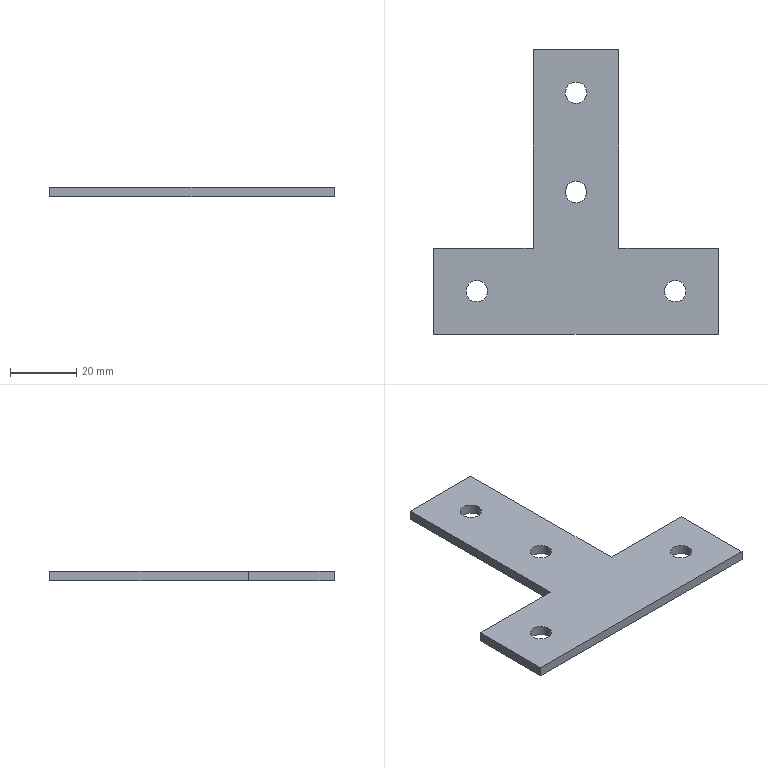Part | STEP file | Outer connecting plate L | 1 solid | 18 faces | box 86 x 86 x 3 mm | volume 10990 mm3 | plane 10 | cylinder 8 | commonest cylinder face diameters 6.5 x8
STEP:
#1=CARTESIAN_POINT('',(0.,0.,0.));
#2=DIRECTION('',(0.,0.,1.));
#3=DIRECTION('',(1.,0.,0.));
#4=AXIS2_PLACEMENT_3D('',#1,#2,#3);
#5=CARTESIAN_POINT('',(3.25,73.,0.));
#6=VERTEX_POINT('',#5);
#7=CARTESIAN_POINT('',(3.25,73.,3.));
#8=VERTEX_POINT('',#7);
#9=CARTESIAN_POINT('',(3.25,73.,3.));
#10=DIRECTION('',(0.,0.,1.));
#11=VECTOR('',#10,1.);
#12=LINE('',#9,#11);
#13=CARTESIAN_POINT('',(0.,73.,3.));
#14=DIRECTION('',(0.,0.,1.));
#15=DIRECTION('',(1.,0.,0.));
#16=AXIS2_PLACEMENT_3D('',#13,#14,#15);
#17=CYLINDRICAL_SURFACE('',#16,3.25);
#18=CARTESIAN_POINT('',(6.283,0.));
#19=DIRECTION('',(0.,1.));
#20=VECTOR('',#19,1.);
#21=LINE('',#18,#20);
#22=(GEOMETRIC_REPRESENTATION_CONTEXT(2)PARAMETRIC_REPRESENTATION_CONTEXT()REPRESENTATION_CONTEXT('',''));
#23=DEFINITIONAL_REPRESENTATION('',(#21),#22);
#24=PCURVE('',#17,#23);
#25=CARTESIAN_POINT('',(0.,73.,3.));
#26=DIRECTION('',(0.,0.,1.));
#27=DIRECTION('',(1.,0.,0.));
#28=AXIS2_PLACEMENT_3D('',#25,#26,#27);
#29=CYLINDRICAL_SURFACE('',#28,3.25);
#30=CARTESIAN_POINT('',(0.,0.));
#31=DIRECTION('',(0.,1.));
#32=VECTOR('',#31,1.);
#33=LINE('',#30,#32);
#34=(GEOMETRIC_REPRESENTATION_CONTEXT(2)PARAMETRIC_REPRESENTATION_CONTEXT()REPRESENTATION_CONTEXT('',''));
#35=DEFINITIONAL_REPRESENTATION('',(#33),#34);
#36=PCURVE('',#29,#35);
#37=SURFACE_CURVE('',#12,(#24,#36),.PCURVE_S1.);
#38=EDGE_CURVE('',#6,#8,#37,.T.);
#39=ORIENTED_EDGE('',*,*,#38,.T.);
#40=CARTESIAN_POINT('',(-3.25,73.,3.));
#41=VERTEX_POINT('',#40);
#42=CARTESIAN_POINT('',(0.,73.,3.));
#43=DIRECTION('',(0.,0.,1.));
#44=DIRECTION('',(1.,0.,0.));
#45=AXIS2_PLACEMENT_3D('',#42,#43,#44);
#46=CIRCLE('',#45,3.25);
#47=CARTESIAN_POINT('',(0.,0.));
#48=DIRECTION('',(1.,0.));
#49=VECTOR('',#48,1.);
#50=LINE('',#47,#49);
#51=(GEOMETRIC_REPRESENTATION_CONTEXT(2)PARAMETRIC_REPRESENTATION_CONTEXT()REPRESENTATION_CONTEXT('',''));
#52=DEFINITIONAL_REPRESENTATION('',(#50),#51);
#53=PCURVE('',#17,#52);
#54=CARTESIAN_POINT('',(0.,0.,3.));
#55=DIRECTION('',(0.,0.,-1.));
#56=DIRECTION('',(-1.,0.,0.));
#57=AXIS2_PLACEMENT_3D('',#54,#55,#56);
#58=PLANE('',#57);
#59=CARTESIAN_POINT('',(-3.25,73.));
#60=CARTESIAN_POINT('',(-3.25,78.629));
#61=CARTESIAN_POINT('',(1.625,75.815));
#62=CARTESIAN_POINT('',(6.5,73.));
#63=CARTESIAN_POINT('',(1.625,70.185));
#64=CARTESIAN_POINT('',(-3.25,67.371));
#65=CARTESIAN_POINT('',(-3.25,73.));
#66=(BOUNDED_CURVE()B_SPLINE_CURVE(2,(#59,#60,#61,#62,#63,#64,#65),.UNSPECIFIED.,.T.,.F.)B_SPLINE_CURVE_WITH_KNOTS((1,2,2,2,2,1),(-2.094,0.,2.094,4.189,6.283,8.378),.UNSPECIFIED.)CURVE()GEOMETRIC_REPRESENTATION_ITEM()RATIONAL_B_SPLINE_CURVE((1.,0.5,1.,0.5,1.,0.5,1.))REPRESENTATION_ITEM(''));
#67=(GEOMETRIC_REPRESENTATION_CONTEXT(2)PARAMETRIC_REPRESENTATION_CONTEXT()REPRESENTATION_CONTEXT('',''));
#68=DEFINITIONAL_REPRESENTATION('',(#66),#67);
#69=PCURVE('',#58,#68);
#70=SURFACE_CURVE('',#46,(#53,#69),.PCURVE_S1.);
#71=EDGE_CURVE('',#41,#8,#70,.T.);
#72=ORIENTED_EDGE('',*,*,#71,.F.);
#73=CARTESIAN_POINT('',(-3.25,73.,0.));
#74=VERTEX_POINT('',#73);
#75=CARTESIAN_POINT('',(-3.25,73.,3.));
#76=DIRECTION('',(0.,0.,1.));
#77=VECTOR('',#76,1.);
#78=LINE('',#75,#77);
#79=CARTESIAN_POINT('',(3.142,0.));
#80=DIRECTION('',(0.,1.));
#81=VECTOR('',#80,1.);
#82=LINE('',#79,#81);
#83=(GEOMETRIC_REPRESENTATION_CONTEXT(2)PARAMETRIC_REPRESENTATION_CONTEXT()REPRESENTATION_CONTEXT('',''));
#84=DEFINITIONAL_REPRESENTATION('',(#82),#83);
#85=PCURVE('',#17,#84);
#86=CARTESIAN_POINT('',(3.142,0.));
#87=DIRECTION('',(0.,1.));
#88=VECTOR('',#87,1.);
#89=LINE('',#86,#88);
#90=(GEOMETRIC_REPRESENTATION_CONTEXT(2)PARAMETRIC_REPRESENTATION_CONTEXT()REPRESENTATION_CONTEXT('',''));
#91=DEFINITIONAL_REPRESENTATION('',(#89),#90);
#92=PCURVE('',#29,#91);
#93=SURFACE_CURVE('',#78,(#85,#92),.PCURVE_S1.);
#94=EDGE_CURVE('',#74,#41,#93,.T.);
#95=ORIENTED_EDGE('',*,*,#94,.F.);
#96=CARTESIAN_POINT('',(0.,73.,0.));
#97=DIRECTION('',(0.,0.,1.));
#98=DIRECTION('',(1.,0.,0.));
#99=AXIS2_PLACEMENT_3D('',#96,#97,#98);
#100=CIRCLE('',#99,3.25);
#101=CARTESIAN_POINT('',(0.,-3.));
#102=DIRECTION('',(1.,0.));
#103=VECTOR('',#102,1.);
#104=LINE('',#101,#103);
#105=(GEOMETRIC_REPRESENTATION_CONTEXT(2)PARAMETRIC_REPRESENTATION_CONTEXT()REPRESENTATION_CONTEXT('',''));
#106=DEFINITIONAL_REPRESENTATION('',(#104),#105);
#107=PCURVE('',#17,#106);
#108=CARTESIAN_POINT('',(0.,0.,0.));
#109=DIRECTION('',(0.,0.,-1.));
#110=DIRECTION('',(-1.,0.,0.));
#111=AXIS2_PLACEMENT_3D('',#108,#109,#110);
#112=PLANE('',#111);
#113=CARTESIAN_POINT('',(-3.25,73.));
#114=CARTESIAN_POINT('',(-3.25,78.629));
#115=CARTESIAN_POINT('',(1.625,75.815));
#116=CARTESIAN_POINT('',(6.5,73.));
#117=CARTESIAN_POINT('',(1.625,70.185));
#118=CARTESIAN_POINT('',(-3.25,67.371));
#119=CARTESIAN_POINT('',(-3.25,73.));
#120=(BOUNDED_CURVE()B_SPLINE_CURVE(2,(#113,#114,#115,#116,#117,#118,#119),.UNSPECIFIED.,.T.,.F.)B_SPLINE_CURVE_WITH_KNOTS((1,2,2,2,2,1),(-2.094,0.,2.094,4.189,6.283,8.378),.UNSPECIFIED.)CURVE()GEOMETRIC_REPRESENTATION_ITEM()RATIONAL_B_SPLINE_CURVE((1.,0.5,1.,0.5,1.,0.5,1.))REPRESENTATION_ITEM(''));
#121=(GEOMETRIC_REPRESENTATION_CONTEXT(2)PARAMETRIC_REPRESENTATION_CONTEXT()REPRESENTATION_CONTEXT('',''));
#122=DEFINITIONAL_REPRESENTATION('',(#120),#121);
#123=PCURVE('',#112,#122);
#124=SURFACE_CURVE('',#100,(#107,#123),.PCURVE_S1.);
#125=EDGE_CURVE('',#74,#6,#124,.T.);
#126=ORIENTED_EDGE('',*,*,#125,.T.);
#127=EDGE_LOOP('',(#39,#72,#95,#126));
#128=FACE_BOUND('',#127,.F.);
#129=ADVANCED_FACE('',(#128),#17,.F.);
#130=CARTESIAN_POINT('',(3.25,43.,0.));
#131=VERTEX_POINT('',#130);
#132=CARTESIAN_POINT('',(3.25,43.,3.));
#133=VERTEX_POINT('',#132);
#134=CARTESIAN_POINT('',(3.25,43.,3.));
#135=DIRECTION('',(0.,0.,1.));
#136=VECTOR('',#135,1.);
#137=LINE('',#134,#136);
#138=CARTESIAN_POINT('',(0.,43.,3.));
#139=DIRECTION('',(0.,0.,1.));
#140=DIRECTION('',(1.,0.,0.));
#141=AXIS2_PLACEMENT_3D('',#138,#139,#140);
#142=CYLINDRICAL_SURFACE('',#141,3.25);
#143=CARTESIAN_POINT('',(6.283,0.));
#144=DIRECTION('',(0.,1.));
#145=VECTOR('',#144,1.);
#146=LINE('',#143,#145);
#147=(GEOMETRIC_REPRESENTATION_CONTEXT(2)PARAMETRIC_REPRESENTATION_CONTEXT()REPRESENTATION_CONTEXT('',''));
#148=DEFINITIONAL_REPRESENTATION('',(#146),#147);
#149=PCURVE('',#142,#148);
#150=CARTESIAN_POINT('',(0.,43.,3.));
#151=DIRECTION('',(0.,0.,1.));
#152=DIRECTION('',(1.,0.,0.));
#153=AXIS2_PLACEMENT_3D('',#150,#151,#152);
#154=CYLINDRICAL_SURFACE('',#153,3.25);
#155=CARTESIAN_POINT('',(0.,0.));
#156=DIRECTION('',(0.,1.));
#157=VECTOR('',#156,1.);
#158=LINE('',#155,#157);
#159=(GEOMETRIC_REPRESENTATION_CONTEXT(2)PARAMETRIC_REPRESENTATION_CONTEXT()REPRESENTATION_CONTEXT('',''));
#160=DEFINITIONAL_REPRESENTATION('',(#158),#159);
#161=PCURVE('',#154,#160);
#162=SURFACE_CURVE('',#137,(#149,#161),.PCURVE_S1.);
#163=EDGE_CURVE('',#131,#133,#162,.T.);
#164=ORIENTED_EDGE('',*,*,#163,.T.);
#165=CARTESIAN_POINT('',(-3.25,43.,3.));
#166=VERTEX_POINT('',#165);
#167=CARTESIAN_POINT('',(0.,43.,3.));
#168=DIRECTION('',(0.,0.,1.));
#169=DIRECTION('',(1.,0.,0.));
#170=AXIS2_PLACEMENT_3D('',#167,#168,#169);
#171=CIRCLE('',#170,3.25);
#172=CARTESIAN_POINT('',(0.,0.));
#173=DIRECTION('',(1.,0.));
#174=VECTOR('',#173,1.);
#175=LINE('',#172,#174);
#176=(GEOMETRIC_REPRESENTATION_CONTEXT(2)PARAMETRIC_REPRESENTATION_CONTEXT()REPRESENTATION_CONTEXT('',''));
#177=DEFINITIONAL_REPRESENTATION('',(#175),#176);
#178=PCURVE('',#142,#177);
#179=CARTESIAN_POINT('',(-3.25,43.));
#180=CARTESIAN_POINT('',(-3.25,48.629));
#181=CARTESIAN_POINT('',(1.625,45.815));
#182=CARTESIAN_POINT('',(6.5,43.));
#183=CARTESIAN_POINT('',(1.625,40.185));
#184=CARTESIAN_POINT('',(-3.25,37.371));
#185=CARTESIAN_POINT('',(-3.25,43.));
#186=(BOUNDED_CURVE()B_SPLINE_CURVE(2,(#179,#180,#181,#182,#183,#184,#185),.UNSPECIFIED.,.T.,.F.)B_SPLINE_CURVE_WITH_KNOTS((1,2,2,2,2,1),(-2.094,0.,2.094,4.189,6.283,8.378),.UNSPECIFIED.)CURVE()GEOMETRIC_REPRESENTATION_ITEM()RATIONAL_B_SPLINE_CURVE((1.,0.5,1.,0.5,1.,0.5,1.))REPRESENTATION_ITEM(''));
#187=(GEOMETRIC_REPRESENTATION_CONTEXT(2)PARAMETRIC_REPRESENTATION_CONTEXT()REPRESENTATION_CONTEXT('',''));
#188=DEFINITIONAL_REPRESENTATION('',(#186),#187);
#189=PCURVE('',#58,#188);
#190=SURFACE_CURVE('',#171,(#178,#189),.PCURVE_S1.);
#191=EDGE_CURVE('',#166,#133,#190,.T.);
#192=ORIENTED_EDGE('',*,*,#191,.F.);
#193=CARTESIAN_POINT('',(-3.25,43.,0.));
#194=VERTEX_POINT('',#193);
#195=CARTESIAN_POINT('',(-3.25,43.,3.));
#196=DIRECTION('',(0.,0.,1.));
#197=VECTOR('',#196,1.);
#198=LINE('',#195,#197);
#199=CARTESIAN_POINT('',(3.142,0.));
#200=DIRECTION('',(0.,1.));
#201=VECTOR('',#200,1.);
#202=LINE('',#199,#201);
#203=(GEOMETRIC_REPRESENTATION_CONTEXT(2)PARAMETRIC_REPRESENTATION_CONTEXT()REPRESENTATION_CONTEXT('',''));
#204=DEFINITIONAL_REPRESENTATION('',(#202),#203);
#205=PCURVE('',#142,#204);
#206=CARTESIAN_POINT('',(3.142,0.));
#207=DIRECTION('',(0.,1.));
#208=VECTOR('',#207,1.);
#209=LINE('',#206,#208);
#210=(GEOMETRIC_REPRESENTATION_CONTEXT(2)PARAMETRIC_REPRESENTATION_CONTEXT()REPRESENTATION_CONTEXT('',''));
#211=DEFINITIONAL_REPRESENTATION('',(#209),#210);
#212=PCURVE('',#154,#211);
#213=SURFACE_CURVE('',#198,(#205,#212),.PCURVE_S1.);
#214=EDGE_CURVE('',#194,#166,#213,.T.);
#215=ORIENTED_EDGE('',*,*,#214,.F.);
#216=CARTESIAN_POINT('',(0.,43.,0.));
#217=DIRECTION('',(0.,0.,1.));
#218=DIRECTION('',(1.,0.,0.));
#219=AXIS2_PLACEMENT_3D('',#216,#217,#218);
#220=CIRCLE('',#219,3.25);
#221=CARTESIAN_POINT('',(0.,-3.));
#222=DIRECTION('',(1.,0.));
#223=VECTOR('',#222,1.);
#224=LINE('',#221,#223);
#225=(GEOMETRIC_REPRESENTATION_CONTEXT(2)PARAMETRIC_REPRESENTATION_CONTEXT()REPRESENTATION_CONTEXT('',''));
#226=DEFINITIONAL_REPRESENTATION('',(#224),#225);
#227=PCURVE('',#142,#226);
#228=CARTESIAN_POINT('',(-3.25,43.));
#229=CARTESIAN_POINT('',(-3.25,48.629));
#230=CARTESIAN_POINT('',(1.625,45.815));
#231=CARTESIAN_POINT('',(6.5,43.));
#232=CARTESIAN_POINT('',(1.625,40.185));
#233=CARTESIAN_POINT('',(-3.25,37.371));
#234=CARTESIAN_POINT('',(-3.25,43.));
#235=(BOUNDED_CURVE()B_SPLINE_CURVE(2,(#228,#229,#230,#231,#232,#233,#234),.UNSPECIFIED.,.T.,.F.)B_SPLINE_CURVE_WITH_KNOTS((1,2,2,2,2,1),(-2.094,0.,2.094,4.189,6.283,8.378),.UNSPECIFIED.)CURVE()GEOMETRIC_REPRESENTATION_ITEM()RATIONAL_B_SPLINE_CURVE((1.,0.5,1.,0.5,1.,0.5,1.))REPRESENTATION_ITEM(''));
#236=(GEOMETRIC_REPRESENTATION_CONTEXT(2)PARAMETRIC_REPRESENTATION_CONTEXT()REPRESENTATION_CONTEXT('',''));
#237=DEFINITIONAL_REPRESENTATION('',(#235),#236);
#238=PCURVE('',#112,#237);
#239=SURFACE_CURVE('',#220,(#227,#238),.PCURVE_S1.);
#240=EDGE_CURVE('',#194,#131,#239,.T.);
#241=ORIENTED_EDGE('',*,*,#240,.T.);
#242=EDGE_LOOP('',(#164,#192,#215,#241));
#243=FACE_BOUND('',#242,.F.);
#244=ADVANCED_FACE('',(#243),#142,.F.);
#245=CARTESIAN_POINT('',(-26.75,13.,0.));
#246=VERTEX_POINT('',#245);
#247=CARTESIAN_POINT('',(-26.75,13.,3.));
#248=VERTEX_POINT('',#247);
#249=CARTESIAN_POINT('',(-26.75,13.,3.));
#250=DIRECTION('',(0.,0.,1.));
#251=VECTOR('',#250,1.);
#252=LINE('',#249,#251);
#253=CARTESIAN_POINT('',(-30.,13.,3.));
#254=DIRECTION('',(0.,0.,1.));
#255=DIRECTION('',(1.,0.,0.));
#256=AXIS2_PLACEMENT_3D('',#253,#254,#255);
#257=CYLINDRICAL_SURFACE('',#256,3.25);
#258=CARTESIAN_POINT('',(6.283,0.));
#259=DIRECTION('',(0.,1.));
#260=VECTOR('',#259,1.);
#261=LINE('',#258,#260);
#262=(GEOMETRIC_REPRESENTATION_CONTEXT(2)PARAMETRIC_REPRESENTATION_CONTEXT()REPRESENTATION_CONTEXT('',''));
#263=DEFINITIONAL_REPRESENTATION('',(#261),#262);
#264=PCURVE('',#257,#263);
#265=CARTESIAN_POINT('',(-30.,13.,3.));
#266=DIRECTION('',(0.,0.,1.));
#267=DIRECTION('',(1.,0.,0.));
#268=AXIS2_PLACEMENT_3D('',#265,#266,#267);
#269=CYLINDRICAL_SURFACE('',#268,3.25);
#270=CARTESIAN_POINT('',(0.,0.));
#271=DIRECTION('',(0.,1.));
#272=VECTOR('',#271,1.);
#273=LINE('',#270,#272);
#274=(GEOMETRIC_REPRESENTATION_CONTEXT(2)PARAMETRIC_REPRESENTATION_CONTEXT()REPRESENTATION_CONTEXT('',''));
#275=DEFINITIONAL_REPRESENTATION('',(#273),#274);
#276=PCURVE('',#269,#275);
#277=SURFACE_CURVE('',#252,(#264,#276),.PCURVE_S1.);
#278=EDGE_CURVE('',#246,#248,#277,.T.);
#279=ORIENTED_EDGE('',*,*,#278,.T.);
#280=CARTESIAN_POINT('',(-33.25,13.,3.));
#281=VERTEX_POINT('',#280);
#282=CARTESIAN_POINT('',(-30.,13.,3.));
#283=DIRECTION('',(0.,0.,1.));
#284=DIRECTION('',(1.,0.,0.));
#285=AXIS2_PLACEMENT_3D('',#282,#283,#284);
#286=CIRCLE('',#285,3.25);
#287=CARTESIAN_POINT('',(0.,0.));
#288=DIRECTION('',(1.,0.));
#289=VECTOR('',#288,1.);
#290=LINE('',#287,#289);
#291=(GEOMETRIC_REPRESENTATION_CONTEXT(2)PARAMETRIC_REPRESENTATION_CONTEXT()REPRESENTATION_CONTEXT('',''));
#292=DEFINITIONAL_REPRESENTATION('',(#290),#291);
#293=PCURVE('',#257,#292);
#294=CARTESIAN_POINT('',(26.75,13.));
#295=CARTESIAN_POINT('',(26.75,18.629));
#296=CARTESIAN_POINT('',(31.625,15.815));
#297=CARTESIAN_POINT('',(36.5,13.));
#298=CARTESIAN_POINT('',(31.625,10.185));
#299=CARTESIAN_POINT('',(26.75,7.371));
#300=CARTESIAN_POINT('',(26.75,13.));
#301=(BOUNDED_CURVE()B_SPLINE_CURVE(2,(#294,#295,#296,#297,#298,#299,#300),.UNSPECIFIED.,.T.,.F.)B_SPLINE_CURVE_WITH_KNOTS((1,2,2,2,2,1),(-2.094,0.,2.094,4.189,6.283,8.378),.UNSPECIFIED.)CURVE()GEOMETRIC_REPRESENTATION_ITEM()RATIONAL_B_SPLINE_CURVE((1.,0.5,1.,0.5,1.,0.5,1.))REPRESENTATION_ITEM(''));
#302=(GEOMETRIC_REPRESENTATION_CONTEXT(2)PARAMETRIC_REPRESENTATION_CONTEXT()REPRESENTATION_CONTEXT('',''));
#303=DEFINITIONAL_REPRESENTATION('',(#301),#302);
#304=PCURVE('',#58,#303);
#305=SURFACE_CURVE('',#286,(#293,#304),.PCURVE_S1.);
#306=EDGE_CURVE('',#281,#248,#305,.T.);
#307=ORIENTED_EDGE('',*,*,#306,.F.);
#308=CARTESIAN_POINT('',(-33.25,13.,0.));
#309=VERTEX_POINT('',#308);
#310=CARTESIAN_POINT('',(-33.25,13.,3.));
#311=DIRECTION('',(0.,0.,1.));
#312=VECTOR('',#311,1.);
#313=LINE('',#310,#312);
#314=CARTESIAN_POINT('',(3.142,0.));
#315=DIRECTION('',(0.,1.));
#316=VECTOR('',#315,1.);
#317=LINE('',#314,#316);
#318=(GEOMETRIC_REPRESENTATION_CONTEXT(2)PARAMETRIC_REPRESENTATION_CONTEXT()REPRESENTATION_CONTEXT('',''));
#319=DEFINITIONAL_REPRESENTATION('',(#317),#318);
#320=PCURVE('',#257,#319);
#321=CARTESIAN_POINT('',(3.142,0.));
#322=DIRECTION('',(0.,1.));
#323=VECTOR('',#322,1.);
#324=LINE('',#321,#323);
#325=(GEOMETRIC_REPRESENTATION_CONTEXT(2)PARAMETRIC_REPRESENTATION_CONTEXT()REPRESENTATION_CONTEXT('',''));
#326=DEFINITIONAL_REPRESENTATION('',(#324),#325);
#327=PCURVE('',#269,#326);
#328=SURFACE_CURVE('',#313,(#320,#327),.PCURVE_S1.);
#329=EDGE_CURVE('',#309,#281,#328,.T.);
#330=ORIENTED_EDGE('',*,*,#329,.F.);
#331=CARTESIAN_POINT('',(-30.,13.,0.));
#332=DIRECTION('',(0.,0.,1.));
#333=DIRECTION('',(1.,0.,0.));
#334=AXIS2_PLACEMENT_3D('',#331,#332,#333);
#335=CIRCLE('',#334,3.25);
#336=CARTESIAN_POINT('',(0.,-3.));
#337=DIRECTION('',(1.,0.));
#338=VECTOR('',#337,1.);
#339=LINE('',#336,#338);
#340=(GEOMETRIC_REPRESENTATION_CONTEXT(2)PARAMETRIC_REPRESENTATION_CONTEXT()REPRESENTATION_CONTEXT('',''));
#341=DEFINITIONAL_REPRESENTATION('',(#339),#340);
#342=PCURVE('',#257,#341);
#343=CARTESIAN_POINT('',(26.75,13.));
#344=CARTESIAN_POINT('',(26.75,18.629));
#345=CARTESIAN_POINT('',(31.625,15.815));
#346=CARTESIAN_POINT('',(36.5,13.));
#347=CARTESIAN_POINT('',(31.625,10.185));
#348=CARTESIAN_POINT('',(26.75,7.371));
#349=CARTESIAN_POINT('',(26.75,13.));
#350=(BOUNDED_CURVE()B_SPLINE_CURVE(2,(#343,#344,#345,#346,#347,#348,#349),.UNSPECIFIED.,.T.,.F.)B_SPLINE_CURVE_WITH_KNOTS((1,2,2,2,2,1),(-2.094,0.,2.094,4.189,6.283,8.378),.UNSPECIFIED.)CURVE()GEOMETRIC_REPRESENTATION_ITEM()RATIONAL_B_SPLINE_CURVE((1.,0.5,1.,0.5,1.,0.5,1.))REPRESENTATION_ITEM(''));
#351=(GEOMETRIC_REPRESENTATION_CONTEXT(2)PARAMETRIC_REPRESENTATION_CONTEXT()REPRESENTATION_CONTEXT('',''));
#352=DEFINITIONAL_REPRESENTATION('',(#350),#351);
#353=PCURVE('',#112,#352);
#354=SURFACE_CURVE('',#335,(#342,#353),.PCURVE_S1.);
#355=EDGE_CURVE('',#309,#246,#354,.T.);
#356=ORIENTED_EDGE('',*,*,#355,.T.);
#357=EDGE_LOOP('',(#279,#307,#330,#356));
#358=FACE_BOUND('',#357,.F.);
#359=ADVANCED_FACE('',(#358),#257,.F.);
#360=CARTESIAN_POINT('',(33.25,13.,0.));
#361=VERTEX_POINT('',#360);
#362=CARTESIAN_POINT('',(33.25,13.,3.));
#363=VERTEX_POINT('',#362);
#364=CARTESIAN_POINT('',(33.25,13.,3.));
#365=DIRECTION('',(0.,0.,1.));
#366=VECTOR('',#365,1.);
#367=LINE('',#364,#366);
#368=CARTESIAN_POINT('',(30.,13.,3.));
#369=DIRECTION('',(0.,0.,1.));
#370=DIRECTION('',(1.,0.,0.));
#371=AXIS2_PLACEMENT_3D('',#368,#369,#370);
#372=CYLINDRICAL_SURFACE('',#371,3.25);
#373=CARTESIAN_POINT('',(6.283,0.));
#374=DIRECTION('',(0.,1.));
#375=VECTOR('',#374,1.);
#376=LINE('',#373,#375);
#377=(GEOMETRIC_REPRESENTATION_CONTEXT(2)PARAMETRIC_REPRESENTATION_CONTEXT()REPRESENTATION_CONTEXT('',''));
#378=DEFINITIONAL_REPRESENTATION('',(#376),#377);
#379=PCURVE('',#372,#378);
#380=CARTESIAN_POINT('',(30.,13.,3.));
#381=DIRECTION('',(0.,0.,1.));
#382=DIRECTION('',(1.,0.,0.));
#383=AXIS2_PLACEMENT_3D('',#380,#381,#382);
#384=CYLINDRICAL_SURFACE('',#383,3.25);
#385=CARTESIAN_POINT('',(0.,0.));
#386=DIRECTION('',(0.,1.));
#387=VECTOR('',#386,1.);
#388=LINE('',#385,#387);
#389=(GEOMETRIC_REPRESENTATION_CONTEXT(2)PARAMETRIC_REPRESENTATION_CONTEXT()REPRESENTATION_CONTEXT('',''));
#390=DEFINITIONAL_REPRESENTATION('',(#388),#389);
#391=PCURVE('',#384,#390);
#392=SURFACE_CURVE('',#367,(#379,#391),.PCURVE_S1.);
#393=EDGE_CURVE('',#361,#363,#392,.T.);
#394=ORIENTED_EDGE('',*,*,#393,.T.);
#395=CARTESIAN_POINT('',(26.75,13.,3.));
#396=VERTEX_POINT('',#395);
#397=CARTESIAN_POINT('',(30.,13.,3.));
#398=DIRECTION('',(0.,0.,1.));
#399=DIRECTION('',(1.,0.,0.));
#400=AXIS2_PLACEMENT_3D('',#397,#398,#399);
#401=CIRCLE('',#400,3.25);
#402=CARTESIAN_POINT('',(0.,0.));
#403=DIRECTION('',(1.,0.));
#404=VECTOR('',#403,1.);
#405=LINE('',#402,#404);
#406=(GEOMETRIC_REPRESENTATION_CONTEXT(2)PARAMETRIC_REPRESENTATION_CONTEXT()REPRESENTATION_CONTEXT('',''));
#407=DEFINITIONAL_REPRESENTATION('',(#405),#406);
#408=PCURVE('',#372,#407);
#409=CARTESIAN_POINT('',(-33.25,13.));
#410=CARTESIAN_POINT('',(-33.25,18.629));
#411=CARTESIAN_POINT('',(-28.375,15.815));
#412=CARTESIAN_POINT('',(-23.5,13.));
#413=CARTESIAN_POINT('',(-28.375,10.185));
#414=CARTESIAN_POINT('',(-33.25,7.371));
#415=CARTESIAN_POINT('',(-33.25,13.));
#416=(BOUNDED_CURVE()B_SPLINE_CURVE(2,(#409,#410,#411,#412,#413,#414,#415),.UNSPECIFIED.,.T.,.F.)B_SPLINE_CURVE_WITH_KNOTS((1,2,2,2,2,1),(-2.094,0.,2.094,4.189,6.283,8.378),.UNSPECIFIED.)CURVE()GEOMETRIC_REPRESENTATION_ITEM()RATIONAL_B_SPLINE_CURVE((1.,0.5,1.,0.5,1.,0.5,1.))REPRESENTATION_ITEM(''));
#417=(GEOMETRIC_REPRESENTATION_CONTEXT(2)PARAMETRIC_REPRESENTATION_CONTEXT()REPRESENTATION_CONTEXT('',''));
#418=DEFINITIONAL_REPRESENTATION('',(#416),#417);
#419=PCURVE('',#58,#418);
#420=SURFACE_CURVE('',#401,(#408,#419),.PCURVE_S1.);
#421=EDGE_CURVE('',#396,#363,#420,.T.);
#422=ORIENTED_EDGE('',*,*,#421,.F.);
#423=CARTESIAN_POINT('',(26.75,13.,0.));
#424=VERTEX_POINT('',#423);
#425=CARTESIAN_POINT('',(26.75,13.,3.));
#426=DIRECTION('',(0.,0.,1.));
#427=VECTOR('',#426,1.);
#428=LINE('',#425,#427);
#429=CARTESIAN_POINT('',(3.142,0.));
#430=DIRECTION('',(0.,1.));
#431=VECTOR('',#430,1.);
#432=LINE('',#429,#431);
#433=(GEOMETRIC_REPRESENTATION_CONTEXT(2)PARAMETRIC_REPRESENTATION_CONTEXT()REPRESENTATION_CONTEXT('',''));
#434=DEFINITIONAL_REPRESENTATION('',(#432),#433);
#435=PCURVE('',#372,#434);
#436=CARTESIAN_POINT('',(3.142,0.));
#437=DIRECTION('',(0.,1.));
#438=VECTOR('',#437,1.);
#439=LINE('',#436,#438);
#440=(GEOMETRIC_REPRESENTATION_CONTEXT(2)PARAMETRIC_REPRESENTATION_CONTEXT()REPRESENTATION_CONTEXT('',''));
#441=DEFINITIONAL_REPRESENTATION('',(#439),#440);
#442=PCURVE('',#384,#441);
#443=SURFACE_CURVE('',#428,(#435,#442),.PCURVE_S1.);
#444=EDGE_CURVE('',#424,#396,#443,.T.);
#445=ORIENTED_EDGE('',*,*,#444,.F.);
#446=CARTESIAN_POINT('',(30.,13.,0.));
#447=DIRECTION('',(0.,0.,1.));
#448=DIRECTION('',(1.,0.,0.));
#449=AXIS2_PLACEMENT_3D('',#446,#447,#448);
#450=CIRCLE('',#449,3.25);
#451=CARTESIAN_POINT('',(0.,-3.));
#452=DIRECTION('',(1.,0.));
#453=VECTOR('',#452,1.);
#454=LINE('',#451,#453);
#455=(GEOMETRIC_REPRESENTATION_CONTEXT(2)PARAMETRIC_REPRESENTATION_CONTEXT()REPRESENTATION_CONTEXT('',''));
#456=DEFINITIONAL_REPRESENTATION('',(#454),#455);
#457=PCURVE('',#372,#456);
#458=CARTESIAN_POINT('',(-33.25,13.));
#459=CARTESIAN_POINT('',(-33.25,18.629));
#460=CARTESIAN_POINT('',(-28.375,15.815));
#461=CARTESIAN_POINT('',(-23.5,13.));
#462=CARTESIAN_POINT('',(-28.375,10.185));
#463=CARTESIAN_POINT('',(-33.25,7.371));
#464=CARTESIAN_POINT('',(-33.25,13.));
#465=(BOUNDED_CURVE()B_SPLINE_CURVE(2,(#458,#459,#460,#461,#462,#463,#464),.UNSPECIFIED.,.T.,.F.)B_SPLINE_CURVE_WITH_KNOTS((1,2,2,2,2,1),(-2.094,0.,2.094,4.189,6.283,8.378),.UNSPECIFIED.)CURVE()GEOMETRIC_REPRESENTATION_ITEM()RATIONAL_B_SPLINE_CURVE((1.,0.5,1.,0.5,1.,0.5,1.))REPRESENTATION_ITEM(''));
#466=(GEOMETRIC_REPRESENTATION_CONTEXT(2)PARAMETRIC_REPRESENTATION_CONTEXT()REPRESENTATION_CONTEXT('',''));
#467=DEFINITIONAL_REPRESENTATION('',(#465),#466);
#468=PCURVE('',#112,#467);
#469=SURFACE_CURVE('',#450,(#457,#468),.PCURVE_S1.);
#470=EDGE_CURVE('',#424,#361,#469,.T.);
#471=ORIENTED_EDGE('',*,*,#470,.T.);
#472=EDGE_LOOP('',(#394,#422,#445,#471));
#473=FACE_BOUND('',#472,.F.);
#474=ADVANCED_FACE('',(#473),#372,.F.);
#475=CARTESIAN_POINT('',(-43.,0.,0.));
#476=VERTEX_POINT('',#475);
#477=CARTESIAN_POINT('',(43.,0.,0.));
#478=VERTEX_POINT('',#477);
#479=CARTESIAN_POINT('',(43.,0.,0.));
#480=DIRECTION('',(1.,0.,0.));
#481=VECTOR('',#480,1.);
#482=LINE('',#479,#481);
#483=CARTESIAN_POINT('',(43.,0.,3.));
#484=DIRECTION('',(0.,1.,0.));
#485=DIRECTION('',(0.,0.,1.));
#486=AXIS2_PLACEMENT_3D('',#483,#484,#485);
#487=PLANE('',#486);
#488=CARTESIAN_POINT('',(-3.,0.));
#489=DIRECTION('',(0.,1.));
#490=VECTOR('',#489,1.);
#491=LINE('',#488,#490);
#492=(GEOMETRIC_REPRESENTATION_CONTEXT(2)PARAMETRIC_REPRESENTATION_CONTEXT()REPRESENTATION_CONTEXT('',''));
#493=DEFINITIONAL_REPRESENTATION('',(#491),#492);
#494=PCURVE('',#487,#493);
#495=CARTESIAN_POINT('',(-43.,0.));
#496=DIRECTION('',(-1.,0.));
#497=VECTOR('',#496,1.);
#498=LINE('',#495,#497);
#499=(GEOMETRIC_REPRESENTATION_CONTEXT(2)PARAMETRIC_REPRESENTATION_CONTEXT()REPRESENTATION_CONTEXT('',''));
#500=DEFINITIONAL_REPRESENTATION('',(#498),#499);
#501=PCURVE('',#112,#500);
#502=SURFACE_CURVE('',#482,(#494,#501),.PCURVE_S1.);
#503=EDGE_CURVE('',#476,#478,#502,.T.);
#504=ORIENTED_EDGE('',*,*,#503,.T.);
#505=CARTESIAN_POINT('',(43.,0.,3.));
#506=VERTEX_POINT('',#505);
#507=CARTESIAN_POINT('',(43.,0.,3.));
#508=DIRECTION('',(0.,0.,-1.));
#509=VECTOR('',#508,1.);
#510=LINE('',#507,#509);
#511=CARTESIAN_POINT('',(0.,0.));
#512=DIRECTION('',(-1.,0.));
#513=VECTOR('',#512,1.);
#514=LINE('',#511,#513);
#515=(GEOMETRIC_REPRESENTATION_CONTEXT(2)PARAMETRIC_REPRESENTATION_CONTEXT()REPRESENTATION_CONTEXT('',''));
#516=DEFINITIONAL_REPRESENTATION('',(#514),#515);
#517=PCURVE('',#487,#516);
#518=CARTESIAN_POINT('',(43.,26.,3.));
#519=DIRECTION('',(-1.,0.,0.));
#520=DIRECTION('',(0.,-1.,0.));
#521=AXIS2_PLACEMENT_3D('',#518,#519,#520);
#522=PLANE('',#521);
#523=CARTESIAN_POINT('',(26.,0.));
#524=DIRECTION('',(0.,-1.));
#525=VECTOR('',#524,1.);
#526=LINE('',#523,#525);
#527=(GEOMETRIC_REPRESENTATION_CONTEXT(2)PARAMETRIC_REPRESENTATION_CONTEXT()REPRESENTATION_CONTEXT('',''));
#528=DEFINITIONAL_REPRESENTATION('',(#526),#527);
#529=PCURVE('',#522,#528);
#530=SURFACE_CURVE('',#510,(#517,#529),.PCURVE_S1.);
#531=EDGE_CURVE('',#506,#478,#530,.T.);
#532=ORIENTED_EDGE('',*,*,#531,.F.);
#533=CARTESIAN_POINT('',(-43.,0.,3.));
#534=VERTEX_POINT('',#533);
#535=CARTESIAN_POINT('',(43.,0.,3.));
#536=DIRECTION('',(1.,0.,0.));
#537=VECTOR('',#536,1.);
#538=LINE('',#535,#537);
#539=CARTESIAN_POINT('',(0.,0.));
#540=DIRECTION('',(0.,1.));
#541=VECTOR('',#540,1.);
#542=LINE('',#539,#541);
#543=(GEOMETRIC_REPRESENTATION_CONTEXT(2)PARAMETRIC_REPRESENTATION_CONTEXT()REPRESENTATION_CONTEXT('',''));
#544=DEFINITIONAL_REPRESENTATION('',(#542),#543);
#545=PCURVE('',#487,#544);
#546=CARTESIAN_POINT('',(-43.,0.));
#547=DIRECTION('',(-1.,0.));
#548=VECTOR('',#547,1.);
#549=LINE('',#546,#548);
#550=(GEOMETRIC_REPRESENTATION_CONTEXT(2)PARAMETRIC_REPRESENTATION_CONTEXT()REPRESENTATION_CONTEXT('',''));
#551=DEFINITIONAL_REPRESENTATION('',(#549),#550);
#552=PCURVE('',#58,#551);
#553=SURFACE_CURVE('',#538,(#545,#552),.PCURVE_S1.);
#554=EDGE_CURVE('',#534,#506,#553,.T.);
#555=ORIENTED_EDGE('',*,*,#554,.F.);
#556=CARTESIAN_POINT('',(-43.,0.,3.));
#557=DIRECTION('',(0.,0.,-1.));
#558=VECTOR('',#557,1.);
#559=LINE('',#556,#558);
#560=CARTESIAN_POINT('',(0.,-86.));
#561=DIRECTION('',(-1.,0.));
#562=VECTOR('',#561,1.);
#563=LINE('',#560,#562);
#564=(GEOMETRIC_REPRESENTATION_CONTEXT(2)PARAMETRIC_REPRESENTATION_CONTEXT()REPRESENTATION_CONTEXT('',''));
#565=DEFINITIONAL_REPRESENTATION('',(#563),#564);
#566=PCURVE('',#487,#565);
#567=CARTESIAN_POINT('',(-43.,0.,3.));
#568=DIRECTION('',(1.,0.,0.));
#569=DIRECTION('',(0.,1.,0.));
#570=AXIS2_PLACEMENT_3D('',#567,#568,#569);
#571=PLANE('',#570);
#572=CARTESIAN_POINT('',(0.,0.));
#573=DIRECTION('',(0.,-1.));
#574=VECTOR('',#573,1.);
#575=LINE('',#572,#574);
#576=(GEOMETRIC_REPRESENTATION_CONTEXT(2)PARAMETRIC_REPRESENTATION_CONTEXT()REPRESENTATION_CONTEXT('',''));
#577=DEFINITIONAL_REPRESENTATION('',(#575),#576);
#578=PCURVE('',#571,#577);
#579=SURFACE_CURVE('',#559,(#566,#578),.PCURVE_S1.);
#580=EDGE_CURVE('',#534,#476,#579,.T.);
#581=ORIENTED_EDGE('',*,*,#580,.T.);
#582=EDGE_LOOP('',(#504,#532,#555,#581));
#583=FACE_BOUND('',#582,.T.);
#584=ADVANCED_FACE('',(#583),#487,.F.);
#585=CARTESIAN_POINT('',(43.,26.,0.));
#586=VERTEX_POINT('',#585);
#587=CARTESIAN_POINT('',(43.,26.,0.));
#588=DIRECTION('',(0.,1.,0.));
#589=VECTOR('',#588,1.);
#590=LINE('',#587,#589);
#591=CARTESIAN_POINT('',(0.,-3.));
#592=DIRECTION('',(-1.,0.));
#593=VECTOR('',#592,1.);
#594=LINE('',#591,#593);
#595=(GEOMETRIC_REPRESENTATION_CONTEXT(2)PARAMETRIC_REPRESENTATION_CONTEXT()REPRESENTATION_CONTEXT('',''));
#596=DEFINITIONAL_REPRESENTATION('',(#594),#595);
#597=PCURVE('',#522,#596);
#598=CARTESIAN_POINT('',(-43.,26.));
#599=DIRECTION('',(0.,1.));
#600=VECTOR('',#599,1.);
#601=LINE('',#598,#600);
#602=(GEOMETRIC_REPRESENTATION_CONTEXT(2)PARAMETRIC_REPRESENTATION_CONTEXT()REPRESENTATION_CONTEXT('',''));
#603=DEFINITIONAL_REPRESENTATION('',(#601),#602);
#604=PCURVE('',#112,#603);
#605=SURFACE_CURVE('',#590,(#597,#604),.PCURVE_S1.);
#606=EDGE_CURVE('',#478,#586,#605,.T.);
#607=ORIENTED_EDGE('',*,*,#606,.T.);
#608=CARTESIAN_POINT('',(43.,26.,3.));
#609=VERTEX_POINT('',#608);
#610=CARTESIAN_POINT('',(43.,26.,3.));
#611=DIRECTION('',(0.,0.,-1.));
#612=VECTOR('',#611,1.);
#613=LINE('',#610,#612);
#614=CARTESIAN_POINT('',(0.,0.));
#615=DIRECTION('',(0.,-1.));
#616=VECTOR('',#615,1.);
#617=LINE('',#614,#616);
#618=(GEOMETRIC_REPRESENTATION_CONTEXT(2)PARAMETRIC_REPRESENTATION_CONTEXT()REPRESENTATION_CONTEXT('',''));
#619=DEFINITIONAL_REPRESENTATION('',(#617),#618);
#620=PCURVE('',#522,#619);
#621=CARTESIAN_POINT('',(13.,26.,3.));
#622=DIRECTION('',(0.,-1.,0.));
#623=DIRECTION('',(1.,0.,0.));
#624=AXIS2_PLACEMENT_3D('',#621,#622,#623);
#625=PLANE('',#624);
#626=CARTESIAN_POINT('',(30.,0.));
#627=DIRECTION('',(0.,-1.));
#628=VECTOR('',#627,1.);
#629=LINE('',#626,#628);
#630=(GEOMETRIC_REPRESENTATION_CONTEXT(2)PARAMETRIC_REPRESENTATION_CONTEXT()REPRESENTATION_CONTEXT('',''));
#631=DEFINITIONAL_REPRESENTATION('',(#629),#630);
#632=PCURVE('',#625,#631);
#633=SURFACE_CURVE('',#613,(#620,#632),.PCURVE_S1.);
#634=EDGE_CURVE('',#609,#586,#633,.T.);
#635=ORIENTED_EDGE('',*,*,#634,.F.);
#636=CARTESIAN_POINT('',(43.,26.,3.));
#637=DIRECTION('',(0.,1.,0.));
#638=VECTOR('',#637,1.);
#639=LINE('',#636,#638);
#640=CARTESIAN_POINT('',(0.,0.));
#641=DIRECTION('',(-1.,0.));
#642=VECTOR('',#641,1.);
#643=LINE('',#640,#642);
#644=(GEOMETRIC_REPRESENTATION_CONTEXT(2)PARAMETRIC_REPRESENTATION_CONTEXT()REPRESENTATION_CONTEXT('',''));
#645=DEFINITIONAL_REPRESENTATION('',(#643),#644);
#646=PCURVE('',#522,#645);
#647=CARTESIAN_POINT('',(-43.,26.));
#648=DIRECTION('',(0.,1.));
#649=VECTOR('',#648,1.);
#650=LINE('',#647,#649);
#651=(GEOMETRIC_REPRESENTATION_CONTEXT(2)PARAMETRIC_REPRESENTATION_CONTEXT()REPRESENTATION_CONTEXT('',''));
#652=DEFINITIONAL_REPRESENTATION('',(#650),#651);
#653=PCURVE('',#58,#652);
#654=SURFACE_CURVE('',#639,(#646,#653),.PCURVE_S1.);
#655=EDGE_CURVE('',#506,#609,#654,.T.);
#656=ORIENTED_EDGE('',*,*,#655,.F.);
#657=ORIENTED_EDGE('',*,*,#531,.T.);
#658=EDGE_LOOP('',(#607,#635,#656,#657));
#659=FACE_BOUND('',#658,.T.);
#660=ADVANCED_FACE('',(#659),#522,.F.);
#661=CARTESIAN_POINT('',(13.,26.,0.));
#662=VERTEX_POINT('',#661);
#663=CARTESIAN_POINT('',(13.,26.,0.));
#664=DIRECTION('',(-1.,0.,0.));
#665=VECTOR('',#664,1.);
#666=LINE('',#663,#665);
#667=CARTESIAN_POINT('',(0.,-3.));
#668=DIRECTION('',(-1.,0.));
#669=VECTOR('',#668,1.);
#670=LINE('',#667,#669);
#671=(GEOMETRIC_REPRESENTATION_CONTEXT(2)PARAMETRIC_REPRESENTATION_CONTEXT()REPRESENTATION_CONTEXT('',''));
#672=DEFINITIONAL_REPRESENTATION('',(#670),#671);
#673=PCURVE('',#625,#672);
#674=CARTESIAN_POINT('',(-13.,26.));
#675=DIRECTION('',(1.,0.));
#676=VECTOR('',#675,1.);
#677=LINE('',#674,#676);
#678=(GEOMETRIC_REPRESENTATION_CONTEXT(2)PARAMETRIC_REPRESENTATION_CONTEXT()REPRESENTATION_CONTEXT('',''));
#679=DEFINITIONAL_REPRESENTATION('',(#677),#678);
#680=PCURVE('',#112,#679);
#681=SURFACE_CURVE('',#666,(#673,#680),.PCURVE_S1.);
#682=EDGE_CURVE('',#586,#662,#681,.T.);
#683=ORIENTED_EDGE('',*,*,#682,.T.);
#684=CARTESIAN_POINT('',(13.,26.,3.));
#685=VERTEX_POINT('',#684);
#686=CARTESIAN_POINT('',(13.,26.,3.));
#687=DIRECTION('',(0.,0.,-1.));
#688=VECTOR('',#687,1.);
#689=LINE('',#686,#688);
#690=CARTESIAN_POINT('',(0.,0.));
#691=DIRECTION('',(0.,-1.));
#692=VECTOR('',#691,1.);
#693=LINE('',#690,#692);
#694=(GEOMETRIC_REPRESENTATION_CONTEXT(2)PARAMETRIC_REPRESENTATION_CONTEXT()REPRESENTATION_CONTEXT('',''));
#695=DEFINITIONAL_REPRESENTATION('',(#693),#694);
#696=PCURVE('',#625,#695);
#697=CARTESIAN_POINT('',(13.,86.,3.));
#698=DIRECTION('',(-1.,0.,0.));
#699=DIRECTION('',(0.,-1.,0.));
#700=AXIS2_PLACEMENT_3D('',#697,#698,#699);
#701=PLANE('',#700);
#702=CARTESIAN_POINT('',(60.,0.));
#703=DIRECTION('',(0.,-1.));
#704=VECTOR('',#703,1.);
#705=LINE('',#702,#704);
#706=(GEOMETRIC_REPRESENTATION_CONTEXT(2)PARAMETRIC_REPRESENTATION_CONTEXT()REPRESENTATION_CONTEXT('',''));
#707=DEFINITIONAL_REPRESENTATION('',(#705),#706);
#708=PCURVE('',#701,#707);
#709=SURFACE_CURVE('',#689,(#696,#708),.PCURVE_S1.);
#710=EDGE_CURVE('',#685,#662,#709,.T.);
#711=ORIENTED_EDGE('',*,*,#710,.F.);
#712=CARTESIAN_POINT('',(13.,26.,3.));
#713=DIRECTION('',(-1.,0.,0.));
#714=VECTOR('',#713,1.);
#715=LINE('',#712,#714);
#716=CARTESIAN_POINT('',(0.,0.));
#717=DIRECTION('',(-1.,0.));
#718=VECTOR('',#717,1.);
#719=LINE('',#716,#718);
#720=(GEOMETRIC_REPRESENTATION_CONTEXT(2)PARAMETRIC_REPRESENTATION_CONTEXT()REPRESENTATION_CONTEXT('',''));
#721=DEFINITIONAL_REPRESENTATION('',(#719),#720);
#722=PCURVE('',#625,#721);
#723=CARTESIAN_POINT('',(-13.,26.));
#724=DIRECTION('',(1.,0.));
#725=VECTOR('',#724,1.);
#726=LINE('',#723,#725);
#727=(GEOMETRIC_REPRESENTATION_CONTEXT(2)PARAMETRIC_REPRESENTATION_CONTEXT()REPRESENTATION_CONTEXT('',''));
#728=DEFINITIONAL_REPRESENTATION('',(#726),#727);
#729=PCURVE('',#58,#728);
#730=SURFACE_CURVE('',#715,(#722,#729),.PCURVE_S1.);
#731=EDGE_CURVE('',#609,#685,#730,.T.);
#732=ORIENTED_EDGE('',*,*,#731,.F.);
#733=ORIENTED_EDGE('',*,*,#634,.T.);
#734=EDGE_LOOP('',(#683,#711,#732,#733));
#735=FACE_BOUND('',#734,.T.);
#736=ADVANCED_FACE('',(#735),#625,.F.);
#737=CARTESIAN_POINT('',(13.,86.,0.));
#738=VERTEX_POINT('',#737);
#739=CARTESIAN_POINT('',(13.,86.,0.));
#740=DIRECTION('',(0.,1.,0.));
#741=VECTOR('',#740,1.);
#742=LINE('',#739,#741);
#743=CARTESIAN_POINT('',(0.,-3.));
#744=DIRECTION('',(-1.,0.));
#745=VECTOR('',#744,1.);
#746=LINE('',#743,#745);
#747=(GEOMETRIC_REPRESENTATION_CONTEXT(2)PARAMETRIC_REPRESENTATION_CONTEXT()REPRESENTATION_CONTEXT('',''));
#748=DEFINITIONAL_REPRESENTATION('',(#746),#747);
#749=PCURVE('',#701,#748);
#750=CARTESIAN_POINT('',(-13.,86.));
#751=DIRECTION('',(0.,1.));
#752=VECTOR('',#751,1.);
#753=LINE('',#750,#752);
#754=(GEOMETRIC_REPRESENTATION_CONTEXT(2)PARAMETRIC_REPRESENTATION_CONTEXT()REPRESENTATION_CONTEXT('',''));
#755=DEFINITIONAL_REPRESENTATION('',(#753),#754);
#756=PCURVE('',#112,#755);
#757=SURFACE_CURVE('',#742,(#749,#756),.PCURVE_S1.);
#758=EDGE_CURVE('',#662,#738,#757,.T.);
#759=ORIENTED_EDGE('',*,*,#758,.T.);
#760=CARTESIAN_POINT('',(13.,86.,3.));
#761=VERTEX_POINT('',#760);
#762=CARTESIAN_POINT('',(13.,86.,3.));
#763=DIRECTION('',(0.,0.,-1.));
#764=VECTOR('',#763,1.);
#765=LINE('',#762,#764);
#766=CARTESIAN_POINT('',(0.,0.));
#767=DIRECTION('',(0.,-1.));
#768=VECTOR('',#767,1.);
#769=LINE('',#766,#768);
#770=(GEOMETRIC_REPRESENTATION_CONTEXT(2)PARAMETRIC_REPRESENTATION_CONTEXT()REPRESENTATION_CONTEXT('',''));
#771=DEFINITIONAL_REPRESENTATION('',(#769),#770);
#772=PCURVE('',#701,#771);
#773=CARTESIAN_POINT('',(-13.,86.,3.));
#774=DIRECTION('',(0.,-1.,0.));
#775=DIRECTION('',(0.,0.,-1.));
#776=AXIS2_PLACEMENT_3D('',#773,#774,#775);
#777=PLANE('',#776);
#778=CARTESIAN_POINT('',(0.,26.));
#779=DIRECTION('',(1.,0.));
#780=VECTOR('',#779,1.);
#781=LINE('',#778,#780);
#782=(GEOMETRIC_REPRESENTATION_CONTEXT(2)PARAMETRIC_REPRESENTATION_CONTEXT()REPRESENTATION_CONTEXT('',''));
#783=DEFINITIONAL_REPRESENTATION('',(#781),#782);
#784=PCURVE('',#777,#783);
#785=SURFACE_CURVE('',#765,(#772,#784),.PCURVE_S1.);
#786=EDGE_CURVE('',#761,#738,#785,.T.);
#787=ORIENTED_EDGE('',*,*,#786,.F.);
#788=CARTESIAN_POINT('',(13.,86.,3.));
#789=DIRECTION('',(0.,1.,0.));
#790=VECTOR('',#789,1.);
#791=LINE('',#788,#790);
#792=CARTESIAN_POINT('',(0.,0.));
#793=DIRECTION('',(-1.,0.));
#794=VECTOR('',#793,1.);
#795=LINE('',#792,#794);
#796=(GEOMETRIC_REPRESENTATION_CONTEXT(2)PARAMETRIC_REPRESENTATION_CONTEXT()REPRESENTATION_CONTEXT('',''));
#797=DEFINITIONAL_REPRESENTATION('',(#795),#796);
#798=PCURVE('',#701,#797);
#799=CARTESIAN_POINT('',(-13.,86.));
#800=DIRECTION('',(0.,1.));
#801=VECTOR('',#800,1.);
#802=LINE('',#799,#801);
#803=(GEOMETRIC_REPRESENTATION_CONTEXT(2)PARAMETRIC_REPRESENTATION_CONTEXT()REPRESENTATION_CONTEXT('',''));
#804=DEFINITIONAL_REPRESENTATION('',(#802),#803);
#805=PCURVE('',#58,#804);
#806=SURFACE_CURVE('',#791,(#798,#805),.PCURVE_S1.);
#807=EDGE_CURVE('',#685,#761,#806,.T.);
#808=ORIENTED_EDGE('',*,*,#807,.F.);
#809=ORIENTED_EDGE('',*,*,#710,.T.);
#810=EDGE_LOOP('',(#759,#787,#808,#809));
#811=FACE_BOUND('',#810,.T.);
#812=ADVANCED_FACE('',(#811),#701,.F.);
#813=CARTESIAN_POINT('',(-13.,86.,0.));
#814=VERTEX_POINT('',#813);
#815=CARTESIAN_POINT('',(-13.,86.,0.));
#816=DIRECTION('',(-1.,0.,0.));
#817=VECTOR('',#816,1.);
#818=LINE('',#815,#817);
#819=CARTESIAN_POINT('',(3.,0.));
#820=DIRECTION('',(0.,-1.));
#821=VECTOR('',#820,1.);
#822=LINE('',#819,#821);
#823=(GEOMETRIC_REPRESENTATION_CONTEXT(2)PARAMETRIC_REPRESENTATION_CONTEXT()REPRESENTATION_CONTEXT('',''));
#824=DEFINITIONAL_REPRESENTATION('',(#822),#823);
#825=PCURVE('',#777,#824);
#826=CARTESIAN_POINT('',(13.,86.));
#827=DIRECTION('',(1.,0.));
#828=VECTOR('',#827,1.);
#829=LINE('',#826,#828);
#830=(GEOMETRIC_REPRESENTATION_CONTEXT(2)PARAMETRIC_REPRESENTATION_CONTEXT()REPRESENTATION_CONTEXT('',''));
#831=DEFINITIONAL_REPRESENTATION('',(#829),#830);
#832=PCURVE('',#112,#831);
#833=SURFACE_CURVE('',#818,(#825,#832),.PCURVE_S1.);
#834=EDGE_CURVE('',#738,#814,#833,.T.);
#835=ORIENTED_EDGE('',*,*,#834,.T.);
#836=CARTESIAN_POINT('',(-13.,86.,3.));
#837=VERTEX_POINT('',#836);
#838=CARTESIAN_POINT('',(-13.,86.,3.));
#839=DIRECTION('',(0.,0.,-1.));
#840=VECTOR('',#839,1.);
#841=LINE('',#838,#840);
#842=CARTESIAN_POINT('',(0.,0.));
#843=DIRECTION('',(1.,0.));
#844=VECTOR('',#843,1.);
#845=LINE('',#842,#844);
#846=(GEOMETRIC_REPRESENTATION_CONTEXT(2)PARAMETRIC_REPRESENTATION_CONTEXT()REPRESENTATION_CONTEXT('',''));
#847=DEFINITIONAL_REPRESENTATION('',(#845),#846);
#848=PCURVE('',#777,#847);
#849=CARTESIAN_POINT('',(-13.,26.,3.));
#850=DIRECTION('',(1.,0.,0.));
#851=DIRECTION('',(0.,1.,0.));
#852=AXIS2_PLACEMENT_3D('',#849,#850,#851);
#853=PLANE('',#852);
#854=CARTESIAN_POINT('',(60.,0.));
#855=DIRECTION('',(0.,-1.));
#856=VECTOR('',#855,1.);
#857=LINE('',#854,#856);
#858=(GEOMETRIC_REPRESENTATION_CONTEXT(2)PARAMETRIC_REPRESENTATION_CONTEXT()REPRESENTATION_CONTEXT('',''));
#859=DEFINITIONAL_REPRESENTATION('',(#857),#858);
#860=PCURVE('',#853,#859);
#861=SURFACE_CURVE('',#841,(#848,#860),.PCURVE_S1.);
#862=EDGE_CURVE('',#837,#814,#861,.T.);
#863=ORIENTED_EDGE('',*,*,#862,.F.);
#864=CARTESIAN_POINT('',(-13.,86.,3.));
#865=DIRECTION('',(-1.,0.,0.));
#866=VECTOR('',#865,1.);
#867=LINE('',#864,#866);
#868=CARTESIAN_POINT('',(0.,0.));
#869=DIRECTION('',(0.,-1.));
#870=VECTOR('',#869,1.);
#871=LINE('',#868,#870);
#872=(GEOMETRIC_REPRESENTATION_CONTEXT(2)PARAMETRIC_REPRESENTATION_CONTEXT()REPRESENTATION_CONTEXT('',''));
#873=DEFINITIONAL_REPRESENTATION('',(#871),#872);
#874=PCURVE('',#777,#873);
#875=CARTESIAN_POINT('',(13.,86.));
#876=DIRECTION('',(1.,0.));
#877=VECTOR('',#876,1.);
#878=LINE('',#875,#877);
#879=(GEOMETRIC_REPRESENTATION_CONTEXT(2)PARAMETRIC_REPRESENTATION_CONTEXT()REPRESENTATION_CONTEXT('',''));
#880=DEFINITIONAL_REPRESENTATION('',(#878),#879);
#881=PCURVE('',#58,#880);
#882=SURFACE_CURVE('',#867,(#874,#881),.PCURVE_S1.);
#883=EDGE_CURVE('',#761,#837,#882,.T.);
#884=ORIENTED_EDGE('',*,*,#883,.F.);
#885=ORIENTED_EDGE('',*,*,#786,.T.);
#886=EDGE_LOOP('',(#835,#863,#884,#885));
#887=FACE_BOUND('',#886,.T.);
#888=ADVANCED_FACE('',(#887),#777,.F.);
#889=CARTESIAN_POINT('',(-13.,26.,0.));
#890=VERTEX_POINT('',#889);
#891=CARTESIAN_POINT('',(-13.,26.,0.));
#892=DIRECTION('',(0.,-1.,0.));
#893=VECTOR('',#892,1.);
#894=LINE('',#891,#893);
#895=CARTESIAN_POINT('',(0.,-3.));
#896=DIRECTION('',(-1.,0.));
#897=VECTOR('',#896,1.);
#898=LINE('',#895,#897);
#899=(GEOMETRIC_REPRESENTATION_CONTEXT(2)PARAMETRIC_REPRESENTATION_CONTEXT()REPRESENTATION_CONTEXT('',''));
#900=DEFINITIONAL_REPRESENTATION('',(#898),#899);
#901=PCURVE('',#853,#900);
#902=CARTESIAN_POINT('',(13.,26.));
#903=DIRECTION('',(0.,-1.));
#904=VECTOR('',#903,1.);
#905=LINE('',#902,#904);
#906=(GEOMETRIC_REPRESENTATION_CONTEXT(2)PARAMETRIC_REPRESENTATION_CONTEXT()REPRESENTATION_CONTEXT('',''));
#907=DEFINITIONAL_REPRESENTATION('',(#905),#906);
#908=PCURVE('',#112,#907);
#909=SURFACE_CURVE('',#894,(#901,#908),.PCURVE_S1.);
#910=EDGE_CURVE('',#814,#890,#909,.T.);
#911=ORIENTED_EDGE('',*,*,#910,.T.);
#912=CARTESIAN_POINT('',(-13.,26.,3.));
#913=VERTEX_POINT('',#912);
#914=CARTESIAN_POINT('',(-13.,26.,3.));
#915=DIRECTION('',(0.,0.,-1.));
#916=VECTOR('',#915,1.);
#917=LINE('',#914,#916);
#918=CARTESIAN_POINT('',(0.,0.));
#919=DIRECTION('',(0.,-1.));
#920=VECTOR('',#919,1.);
#921=LINE('',#918,#920);
#922=(GEOMETRIC_REPRESENTATION_CONTEXT(2)PARAMETRIC_REPRESENTATION_CONTEXT()REPRESENTATION_CONTEXT('',''));
#923=DEFINITIONAL_REPRESENTATION('',(#921),#922);
#924=PCURVE('',#853,#923);
#925=CARTESIAN_POINT('',(-43.,26.,3.));
#926=DIRECTION('',(0.,-1.,0.));
#927=DIRECTION('',(1.,0.,0.));
#928=AXIS2_PLACEMENT_3D('',#925,#926,#927);
#929=PLANE('',#928);
#930=CARTESIAN_POINT('',(30.,0.));
#931=DIRECTION('',(0.,-1.));
#932=VECTOR('',#931,1.);
#933=LINE('',#930,#932);
#934=(GEOMETRIC_REPRESENTATION_CONTEXT(2)PARAMETRIC_REPRESENTATION_CONTEXT()REPRESENTATION_CONTEXT('',''));
#935=DEFINITIONAL_REPRESENTATION('',(#933),#934);
#936=PCURVE('',#929,#935);
#937=SURFACE_CURVE('',#917,(#924,#936),.PCURVE_S1.);
#938=EDGE_CURVE('',#913,#890,#937,.T.);
#939=ORIENTED_EDGE('',*,*,#938,.F.);
#940=CARTESIAN_POINT('',(-13.,26.,3.));
#941=DIRECTION('',(0.,-1.,0.));
#942=VECTOR('',#941,1.);
#943=LINE('',#940,#942);
#944=CARTESIAN_POINT('',(0.,0.));
#945=DIRECTION('',(-1.,0.));
#946=VECTOR('',#945,1.);
#947=LINE('',#944,#946);
#948=(GEOMETRIC_REPRESENTATION_CONTEXT(2)PARAMETRIC_REPRESENTATION_CONTEXT()REPRESENTATION_CONTEXT('',''));
#949=DEFINITIONAL_REPRESENTATION('',(#947),#948);
#950=PCURVE('',#853,#949);
#951=CARTESIAN_POINT('',(13.,26.));
#952=DIRECTION('',(0.,-1.));
#953=VECTOR('',#952,1.);
#954=LINE('',#951,#953);
#955=(GEOMETRIC_REPRESENTATION_CONTEXT(2)PARAMETRIC_REPRESENTATION_CONTEXT()REPRESENTATION_CONTEXT('',''));
#956=DEFINITIONAL_REPRESENTATION('',(#954),#955);
#957=PCURVE('',#58,#956);
#958=SURFACE_CURVE('',#943,(#950,#957),.PCURVE_S1.);
#959=EDGE_CURVE('',#837,#913,#958,.T.);
#960=ORIENTED_EDGE('',*,*,#959,.F.);
#961=ORIENTED_EDGE('',*,*,#862,.T.);
#962=EDGE_LOOP('',(#911,#939,#960,#961));
#963=FACE_BOUND('',#962,.T.);
#964=ADVANCED_FACE('',(#963),#853,.F.);
#965=CARTESIAN_POINT('',(-43.,26.,0.));
#966=VERTEX_POINT('',#965);
#967=CARTESIAN_POINT('',(-43.,26.,0.));
#968=DIRECTION('',(-1.,0.,0.));
#969=VECTOR('',#968,1.);
#970=LINE('',#967,#969);
#971=CARTESIAN_POINT('',(0.,-3.));
#972=DIRECTION('',(-1.,0.));
#973=VECTOR('',#972,1.);
#974=LINE('',#971,#973);
#975=(GEOMETRIC_REPRESENTATION_CONTEXT(2)PARAMETRIC_REPRESENTATION_CONTEXT()REPRESENTATION_CONTEXT('',''));
#976=DEFINITIONAL_REPRESENTATION('',(#974),#975);
#977=PCURVE('',#929,#976);
#978=CARTESIAN_POINT('',(43.,26.));
#979=DIRECTION('',(1.,0.));
#980=VECTOR('',#979,1.);
#981=LINE('',#978,#980);
#982=(GEOMETRIC_REPRESENTATION_CONTEXT(2)PARAMETRIC_REPRESENTATION_CONTEXT()REPRESENTATION_CONTEXT('',''));
#983=DEFINITIONAL_REPRESENTATION('',(#981),#982);
#984=PCURVE('',#112,#983);
#985=SURFACE_CURVE('',#970,(#977,#984),.PCURVE_S1.);
#986=EDGE_CURVE('',#890,#966,#985,.T.);
#987=ORIENTED_EDGE('',*,*,#986,.T.);
#988=CARTESIAN_POINT('',(-43.,26.,3.));
#989=VERTEX_POINT('',#988);
#990=CARTESIAN_POINT('',(-43.,26.,3.));
#991=DIRECTION('',(0.,0.,-1.));
#992=VECTOR('',#991,1.);
#993=LINE('',#990,#992);
#994=CARTESIAN_POINT('',(0.,0.));
#995=DIRECTION('',(0.,-1.));
#996=VECTOR('',#995,1.);
#997=LINE('',#994,#996);
#998=(GEOMETRIC_REPRESENTATION_CONTEXT(2)PARAMETRIC_REPRESENTATION_CONTEXT()REPRESENTATION_CONTEXT('',''));
#999=DEFINITIONAL_REPRESENTATION('',(#997),#998);
#1000=PCURVE('',#929,#999);
#1001=CARTESIAN_POINT('',(26.,0.));
#1002=DIRECTION('',(0.,-1.));
#1003=VECTOR('',#1002,1.);
#1004=LINE('',#1001,#1003);
#1005=(GEOMETRIC_REPRESENTATION_CONTEXT(2)PARAMETRIC_REPRESENTATION_CONTEXT()REPRESENTATION_CONTEXT('',''));
#1006=DEFINITIONAL_REPRESENTATION('',(#1004),#1005);
#1007=PCURVE('',#571,#1006);
#1008=SURFACE_CURVE('',#993,(#1000,#1007),.PCURVE_S1.);
#1009=EDGE_CURVE('',#989,#966,#1008,.T.);
#1010=ORIENTED_EDGE('',*,*,#1009,.F.);
#1011=CARTESIAN_POINT('',(-43.,26.,3.));
#1012=DIRECTION('',(-1.,0.,0.));
#1013=VECTOR('',#1012,1.);
#1014=LINE('',#1011,#1013);
#1015=CARTESIAN_POINT('',(0.,0.));
#1016=DIRECTION('',(-1.,0.));
#1017=VECTOR('',#1016,1.);
#1018=LINE('',#1015,#1017);
#1019=(GEOMETRIC_REPRESENTATION_CONTEXT(2)PARAMETRIC_REPRESENTATION_CONTEXT()REPRESENTATION_CONTEXT('',''));
#1020=DEFINITIONAL_REPRESENTATION('',(#1018),#1019);
#1021=PCURVE('',#929,#1020);
#1022=CARTESIAN_POINT('',(43.,26.));
#1023=DIRECTION('',(1.,0.));
#1024=VECTOR('',#1023,1.);
#1025=LINE('',#1022,#1024);
#1026=(GEOMETRIC_REPRESENTATION_CONTEXT(2)PARAMETRIC_REPRESENTATION_CONTEXT()REPRESENTATION_CONTEXT('',''));
#1027=DEFINITIONAL_REPRESENTATION('',(#1025),#1026);
#1028=PCURVE('',#58,#1027);
#1029=SURFACE_CURVE('',#1014,(#1021,#1028),.PCURVE_S1.);
#1030=EDGE_CURVE('',#913,#989,#1029,.T.);
#1031=ORIENTED_EDGE('',*,*,#1030,.F.);
#1032=ORIENTED_EDGE('',*,*,#938,.T.);
#1033=EDGE_LOOP('',(#987,#1010,#1031,#1032));
#1034=FACE_BOUND('',#1033,.T.);
#1035=ADVANCED_FACE('',(#1034),#929,.F.);
#1036=CARTESIAN_POINT('',(-43.,0.,0.));
#1037=DIRECTION('',(0.,-1.,0.));
#1038=VECTOR('',#1037,1.);
#1039=LINE('',#1036,#1038);
#1040=CARTESIAN_POINT('',(0.,-3.));
#1041=DIRECTION('',(-1.,0.));
#1042=VECTOR('',#1041,1.);
#1043=LINE('',#1040,#1042);
#1044=(GEOMETRIC_REPRESENTATION_CONTEXT(2)PARAMETRIC_REPRESENTATION_CONTEXT()REPRESENTATION_CONTEXT('',''));
#1045=DEFINITIONAL_REPRESENTATION('',(#1043),#1044);
#1046=PCURVE('',#571,#1045);
#1047=CARTESIAN_POINT('',(43.,0.));
#1048=DIRECTION('',(0.,-1.));
#1049=VECTOR('',#1048,1.);
#1050=LINE('',#1047,#1049);
#1051=(GEOMETRIC_REPRESENTATION_CONTEXT(2)PARAMETRIC_REPRESENTATION_CONTEXT()REPRESENTATION_CONTEXT('',''));
#1052=DEFINITIONAL_REPRESENTATION('',(#1050),#1051);
#1053=PCURVE('',#112,#1052);
#1054=SURFACE_CURVE('',#1039,(#1046,#1053),.PCURVE_S1.);
#1055=EDGE_CURVE('',#966,#476,#1054,.T.);
#1056=ORIENTED_EDGE('',*,*,#1055,.T.);
#1057=ORIENTED_EDGE('',*,*,#580,.F.);
#1058=CARTESIAN_POINT('',(-43.,0.,3.));
#1059=DIRECTION('',(0.,-1.,0.));
#1060=VECTOR('',#1059,1.);
#1061=LINE('',#1058,#1060);
#1062=CARTESIAN_POINT('',(0.,0.));
#1063=DIRECTION('',(-1.,0.));
#1064=VECTOR('',#1063,1.);
#1065=LINE('',#1062,#1064);
#1066=(GEOMETRIC_REPRESENTATION_CONTEXT(2)PARAMETRIC_REPRESENTATION_CONTEXT()REPRESENTATION_CONTEXT('',''));
#1067=DEFINITIONAL_REPRESENTATION('',(#1065),#1066);
#1068=PCURVE('',#571,#1067);
#1069=CARTESIAN_POINT('',(43.,0.));
#1070=DIRECTION('',(0.,-1.));
#1071=VECTOR('',#1070,1.);
#1072=LINE('',#1069,#1071);
#1073=(GEOMETRIC_REPRESENTATION_CONTEXT(2)PARAMETRIC_REPRESENTATION_CONTEXT()REPRESENTATION_CONTEXT('',''));
#1074=DEFINITIONAL_REPRESENTATION('',(#1072),#1073);
#1075=PCURVE('',#58,#1074);
#1076=SURFACE_CURVE('',#1061,(#1068,#1075),.PCURVE_S1.);
#1077=EDGE_CURVE('',#989,#534,#1076,.T.);
#1078=ORIENTED_EDGE('',*,*,#1077,.F.);
#1079=ORIENTED_EDGE('',*,*,#1009,.T.);
#1080=EDGE_LOOP('',(#1056,#1057,#1078,#1079));
#1081=FACE_BOUND('',#1080,.T.);
#1082=ADVANCED_FACE('',(#1081),#571,.F.);
#1083=CARTESIAN_POINT('',(0.,73.,3.));
#1084=DIRECTION('',(0.,0.,1.));
#1085=DIRECTION('',(1.,0.,0.));
#1086=AXIS2_PLACEMENT_3D('',#1083,#1084,#1085);
#1087=CIRCLE('',#1086,3.25);
#1088=CARTESIAN_POINT('',(-3.25,73.));
#1089=CARTESIAN_POINT('',(-3.25,78.629));
#1090=CARTESIAN_POINT('',(1.625,75.815));
#1091=CARTESIAN_POINT('',(6.5,73.));
#1092=CARTESIAN_POINT('',(1.625,70.185));
#1093=CARTESIAN_POINT('',(-3.25,67.371));
#1094=CARTESIAN_POINT('',(-3.25,73.));
#1095=(BOUNDED_CURVE()B_SPLINE_CURVE(2,(#1088,#1089,#1090,#1091,#1092,#1093,#1094),.UNSPECIFIED.,.T.,.F.)B_SPLINE_CURVE_WITH_KNOTS((1,2,2,2,2,1),(-2.094,0.,2.094,4.189,6.283,8.378),.UNSPECIFIED.)CURVE()GEOMETRIC_REPRESENTATION_ITEM()RATIONAL_B_SPLINE_CURVE((1.,0.5,1.,0.5,1.,0.5,1.))REPRESENTATION_ITEM(''));
#1096=(GEOMETRIC_REPRESENTATION_CONTEXT(2)PARAMETRIC_REPRESENTATION_CONTEXT()REPRESENTATION_CONTEXT('',''));
#1097=DEFINITIONAL_REPRESENTATION('',(#1095),#1096);
#1098=PCURVE('',#58,#1097);
#1099=CARTESIAN_POINT('',(0.,0.));
#1100=DIRECTION('',(1.,0.));
#1101=VECTOR('',#1100,1.);
#1102=LINE('',#1099,#1101);
#1103=(GEOMETRIC_REPRESENTATION_CONTEXT(2)PARAMETRIC_REPRESENTATION_CONTEXT()REPRESENTATION_CONTEXT('',''));
#1104=DEFINITIONAL_REPRESENTATION('',(#1102),#1103);
#1105=PCURVE('',#29,#1104);
#1106=SURFACE_CURVE('',#1087,(#1098,#1105),.PCURVE_S1.);
#1107=EDGE_CURVE('',#8,#41,#1106,.T.);
#1108=ORIENTED_EDGE('',*,*,#1107,.F.);
#1109=ORIENTED_EDGE('',*,*,#71,.F.);
#1110=EDGE_LOOP('',(#1108,#1109));
#1111=FACE_BOUND('',#1110,.T.);
#1112=CARTESIAN_POINT('',(0.,43.,3.));
#1113=DIRECTION('',(0.,0.,1.));
#1114=DIRECTION('',(1.,0.,0.));
#1115=AXIS2_PLACEMENT_3D('',#1112,#1113,#1114);
#1116=CIRCLE('',#1115,3.25);
#1117=CARTESIAN_POINT('',(-3.25,43.));
#1118=CARTESIAN_POINT('',(-3.25,48.629));
#1119=CARTESIAN_POINT('',(1.625,45.815));
#1120=CARTESIAN_POINT('',(6.5,43.));
#1121=CARTESIAN_POINT('',(1.625,40.185));
#1122=CARTESIAN_POINT('',(-3.25,37.371));
#1123=CARTESIAN_POINT('',(-3.25,43.));
#1124=(BOUNDED_CURVE()B_SPLINE_CURVE(2,(#1117,#1118,#1119,#1120,#1121,#1122,#1123),.UNSPECIFIED.,.T.,.F.)B_SPLINE_CURVE_WITH_KNOTS((1,2,2,2,2,1),(-2.094,0.,2.094,4.189,6.283,8.378),.UNSPECIFIED.)CURVE()GEOMETRIC_REPRESENTATION_ITEM()RATIONAL_B_SPLINE_CURVE((1.,0.5,1.,0.5,1.,0.5,1.))REPRESENTATION_ITEM(''));
#1125=(GEOMETRIC_REPRESENTATION_CONTEXT(2)PARAMETRIC_REPRESENTATION_CONTEXT()REPRESENTATION_CONTEXT('',''));
#1126=DEFINITIONAL_REPRESENTATION('',(#1124),#1125);
#1127=PCURVE('',#58,#1126);
#1128=CARTESIAN_POINT('',(0.,0.));
#1129=DIRECTION('',(1.,0.));
#1130=VECTOR('',#1129,1.);
#1131=LINE('',#1128,#1130);
#1132=(GEOMETRIC_REPRESENTATION_CONTEXT(2)PARAMETRIC_REPRESENTATION_CONTEXT()REPRESENTATION_CONTEXT('',''));
#1133=DEFINITIONAL_REPRESENTATION('',(#1131),#1132);
#1134=PCURVE('',#154,#1133);
#1135=SURFACE_CURVE('',#1116,(#1127,#1134),.PCURVE_S1.);
#1136=EDGE_CURVE('',#133,#166,#1135,.T.);
#1137=ORIENTED_EDGE('',*,*,#1136,.F.);
#1138=ORIENTED_EDGE('',*,*,#191,.F.);
#1139=EDGE_LOOP('',(#1137,#1138));
#1140=FACE_BOUND('',#1139,.T.);
#1141=CARTESIAN_POINT('',(-30.,13.,3.));
#1142=DIRECTION('',(0.,0.,1.));
#1143=DIRECTION('',(1.,0.,0.));
#1144=AXIS2_PLACEMENT_3D('',#1141,#1142,#1143);
#1145=CIRCLE('',#1144,3.25);
#1146=CARTESIAN_POINT('',(26.75,13.));
#1147=CARTESIAN_POINT('',(26.75,18.629));
#1148=CARTESIAN_POINT('',(31.625,15.815));
#1149=CARTESIAN_POINT('',(36.5,13.));
#1150=CARTESIAN_POINT('',(31.625,10.185));
#1151=CARTESIAN_POINT('',(26.75,7.371));
#1152=CARTESIAN_POINT('',(26.75,13.));
#1153=(BOUNDED_CURVE()B_SPLINE_CURVE(2,(#1146,#1147,#1148,#1149,#1150,#1151,#1152),.UNSPECIFIED.,.T.,.F.)B_SPLINE_CURVE_WITH_KNOTS((1,2,2,2,2,1),(-2.094,0.,2.094,4.189,6.283,8.378),.UNSPECIFIED.)CURVE()GEOMETRIC_REPRESENTATION_ITEM()RATIONAL_B_SPLINE_CURVE((1.,0.5,1.,0.5,1.,0.5,1.))REPRESENTATION_ITEM(''));
#1154=(GEOMETRIC_REPRESENTATION_CONTEXT(2)PARAMETRIC_REPRESENTATION_CONTEXT()REPRESENTATION_CONTEXT('',''));
#1155=DEFINITIONAL_REPRESENTATION('',(#1153),#1154);
#1156=PCURVE('',#58,#1155);
#1157=CARTESIAN_POINT('',(0.,0.));
#1158=DIRECTION('',(1.,0.));
#1159=VECTOR('',#1158,1.);
#1160=LINE('',#1157,#1159);
#1161=(GEOMETRIC_REPRESENTATION_CONTEXT(2)PARAMETRIC_REPRESENTATION_CONTEXT()REPRESENTATION_CONTEXT('',''));
#1162=DEFINITIONAL_REPRESENTATION('',(#1160),#1161);
#1163=PCURVE('',#269,#1162);
#1164=SURFACE_CURVE('',#1145,(#1156,#1163),.PCURVE_S1.);
#1165=EDGE_CURVE('',#248,#281,#1164,.T.);
#1166=ORIENTED_EDGE('',*,*,#1165,.F.);
#1167=ORIENTED_EDGE('',*,*,#306,.F.);
#1168=EDGE_LOOP('',(#1166,#1167));
#1169=FACE_BOUND('',#1168,.T.);
#1170=CARTESIAN_POINT('',(30.,13.,3.));
#1171=DIRECTION('',(0.,0.,1.));
#1172=DIRECTION('',(1.,0.,0.));
#1173=AXIS2_PLACEMENT_3D('',#1170,#1171,#1172);
#1174=CIRCLE('',#1173,3.25);
#1175=CARTESIAN_POINT('',(-33.25,13.));
#1176=CARTESIAN_POINT('',(-33.25,18.629));
#1177=CARTESIAN_POINT('',(-28.375,15.815));
#1178=CARTESIAN_POINT('',(-23.5,13.));
#1179=CARTESIAN_POINT('',(-28.375,10.185));
#1180=CARTESIAN_POINT('',(-33.25,7.371));
#1181=CARTESIAN_POINT('',(-33.25,13.));
#1182=(BOUNDED_CURVE()B_SPLINE_CURVE(2,(#1175,#1176,#1177,#1178,#1179,#1180,#1181),.UNSPECIFIED.,.T.,.F.)B_SPLINE_CURVE_WITH_KNOTS((1,2,2,2,2,1),(-2.094,0.,2.094,4.189,6.283,8.378),.UNSPECIFIED.)CURVE()GEOMETRIC_REPRESENTATION_ITEM()RATIONAL_B_SPLINE_CURVE((1.,0.5,1.,0.5,1.,0.5,1.))REPRESENTATION_ITEM(''));
#1183=(GEOMETRIC_REPRESENTATION_CONTEXT(2)PARAMETRIC_REPRESENTATION_CONTEXT()REPRESENTATION_CONTEXT('',''));
#1184=DEFINITIONAL_REPRESENTATION('',(#1182),#1183);
#1185=PCURVE('',#58,#1184);
#1186=CARTESIAN_POINT('',(0.,0.));
#1187=DIRECTION('',(1.,0.));
#1188=VECTOR('',#1187,1.);
#1189=LINE('',#1186,#1188);
#1190=(GEOMETRIC_REPRESENTATION_CONTEXT(2)PARAMETRIC_REPRESENTATION_CONTEXT()REPRESENTATION_CONTEXT('',''));
#1191=DEFINITIONAL_REPRESENTATION('',(#1189),#1190);
#1192=PCURVE('',#384,#1191);
#1193=SURFACE_CURVE('',#1174,(#1185,#1192),.PCURVE_S1.);
#1194=EDGE_CURVE('',#363,#396,#1193,.T.);
#1195=ORIENTED_EDGE('',*,*,#1194,.F.);
#1196=ORIENTED_EDGE('',*,*,#421,.F.);
#1197=EDGE_LOOP('',(#1195,#1196));
#1198=FACE_BOUND('',#1197,.T.);
#1199=ORIENTED_EDGE('',*,*,#554,.T.);
#1200=ORIENTED_EDGE('',*,*,#655,.T.);
#1201=ORIENTED_EDGE('',*,*,#731,.T.);
#1202=ORIENTED_EDGE('',*,*,#807,.T.);
#1203=ORIENTED_EDGE('',*,*,#883,.T.);
#1204=ORIENTED_EDGE('',*,*,#959,.T.);
#1205=ORIENTED_EDGE('',*,*,#1030,.T.);
#1206=ORIENTED_EDGE('',*,*,#1077,.T.);
#1207=EDGE_LOOP('',(#1199,#1200,#1201,#1202,#1203,#1204,#1205,#1206));
#1208=FACE_BOUND('',#1207,.T.);
#1209=ADVANCED_FACE('',(#1111,#1140,#1169,#1198,#1208),#58,.F.);
#1210=CARTESIAN_POINT('',(0.,73.,0.));
#1211=DIRECTION('',(0.,0.,1.));
#1212=DIRECTION('',(1.,0.,0.));
#1213=AXIS2_PLACEMENT_3D('',#1210,#1211,#1212);
#1214=CIRCLE('',#1213,3.25);
#1215=CARTESIAN_POINT('',(-3.25,73.));
#1216=CARTESIAN_POINT('',(-3.25,78.629));
#1217=CARTESIAN_POINT('',(1.625,75.815));
#1218=CARTESIAN_POINT('',(6.5,73.));
#1219=CARTESIAN_POINT('',(1.625,70.185));
#1220=CARTESIAN_POINT('',(-3.25,67.371));
#1221=CARTESIAN_POINT('',(-3.25,73.));
#1222=(BOUNDED_CURVE()B_SPLINE_CURVE(2,(#1215,#1216,#1217,#1218,#1219,#1220,#1221),.UNSPECIFIED.,.T.,.F.)B_SPLINE_CURVE_WITH_KNOTS((1,2,2,2,2,1),(-2.094,0.,2.094,4.189,6.283,8.378),.UNSPECIFIED.)CURVE()GEOMETRIC_REPRESENTATION_ITEM()RATIONAL_B_SPLINE_CURVE((1.,0.5,1.,0.5,1.,0.5,1.))REPRESENTATION_ITEM(''));
#1223=(GEOMETRIC_REPRESENTATION_CONTEXT(2)PARAMETRIC_REPRESENTATION_CONTEXT()REPRESENTATION_CONTEXT('',''));
#1224=DEFINITIONAL_REPRESENTATION('',(#1222),#1223);
#1225=PCURVE('',#112,#1224);
#1226=CARTESIAN_POINT('',(0.,-3.));
#1227=DIRECTION('',(1.,0.));
#1228=VECTOR('',#1227,1.);
#1229=LINE('',#1226,#1228);
#1230=(GEOMETRIC_REPRESENTATION_CONTEXT(2)PARAMETRIC_REPRESENTATION_CONTEXT()REPRESENTATION_CONTEXT('',''));
#1231=DEFINITIONAL_REPRESENTATION('',(#1229),#1230);
#1232=PCURVE('',#29,#1231);
#1233=SURFACE_CURVE('',#1214,(#1225,#1232),.PCURVE_S1.);
#1234=EDGE_CURVE('',#6,#74,#1233,.T.);
#1235=ORIENTED_EDGE('',*,*,#1234,.T.);
#1236=ORIENTED_EDGE('',*,*,#125,.T.);
#1237=EDGE_LOOP('',(#1235,#1236));
#1238=FACE_BOUND('',#1237,.T.);
#1239=CARTESIAN_POINT('',(0.,43.,0.));
#1240=DIRECTION('',(0.,0.,1.));
#1241=DIRECTION('',(1.,0.,0.));
#1242=AXIS2_PLACEMENT_3D('',#1239,#1240,#1241);
#1243=CIRCLE('',#1242,3.25);
#1244=CARTESIAN_POINT('',(-3.25,43.));
#1245=CARTESIAN_POINT('',(-3.25,48.629));
#1246=CARTESIAN_POINT('',(1.625,45.815));
#1247=CARTESIAN_POINT('',(6.5,43.));
#1248=CARTESIAN_POINT('',(1.625,40.185));
#1249=CARTESIAN_POINT('',(-3.25,37.371));
#1250=CARTESIAN_POINT('',(-3.25,43.));
#1251=(BOUNDED_CURVE()B_SPLINE_CURVE(2,(#1244,#1245,#1246,#1247,#1248,#1249,#1250),.UNSPECIFIED.,.T.,.F.)B_SPLINE_CURVE_WITH_KNOTS((1,2,2,2,2,1),(-2.094,0.,2.094,4.189,6.283,8.378),.UNSPECIFIED.)CURVE()GEOMETRIC_REPRESENTATION_ITEM()RATIONAL_B_SPLINE_CURVE((1.,0.5,1.,0.5,1.,0.5,1.))REPRESENTATION_ITEM(''));
#1252=(GEOMETRIC_REPRESENTATION_CONTEXT(2)PARAMETRIC_REPRESENTATION_CONTEXT()REPRESENTATION_CONTEXT('',''));
#1253=DEFINITIONAL_REPRESENTATION('',(#1251),#1252);
#1254=PCURVE('',#112,#1253);
#1255=CARTESIAN_POINT('',(0.,-3.));
#1256=DIRECTION('',(1.,0.));
#1257=VECTOR('',#1256,1.);
#1258=LINE('',#1255,#1257);
#1259=(GEOMETRIC_REPRESENTATION_CONTEXT(2)PARAMETRIC_REPRESENTATION_CONTEXT()REPRESENTATION_CONTEXT('',''));
#1260=DEFINITIONAL_REPRESENTATION('',(#1258),#1259);
#1261=PCURVE('',#154,#1260);
#1262=SURFACE_CURVE('',#1243,(#1254,#1261),.PCURVE_S1.);
#1263=EDGE_CURVE('',#131,#194,#1262,.T.);
#1264=ORIENTED_EDGE('',*,*,#1263,.T.);
#1265=ORIENTED_EDGE('',*,*,#240,.T.);
#1266=EDGE_LOOP('',(#1264,#1265));
#1267=FACE_BOUND('',#1266,.T.);
#1268=CARTESIAN_POINT('',(-30.,13.,0.));
#1269=DIRECTION('',(0.,0.,1.));
#1270=DIRECTION('',(1.,0.,0.));
#1271=AXIS2_PLACEMENT_3D('',#1268,#1269,#1270);
#1272=CIRCLE('',#1271,3.25);
#1273=CARTESIAN_POINT('',(26.75,13.));
#1274=CARTESIAN_POINT('',(26.75,18.629));
#1275=CARTESIAN_POINT('',(31.625,15.815));
#1276=CARTESIAN_POINT('',(36.5,13.));
#1277=CARTESIAN_POINT('',(31.625,10.185));
#1278=CARTESIAN_POINT('',(26.75,7.371));
#1279=CARTESIAN_POINT('',(26.75,13.));
#1280=(BOUNDED_CURVE()B_SPLINE_CURVE(2,(#1273,#1274,#1275,#1276,#1277,#1278,#1279),.UNSPECIFIED.,.T.,.F.)B_SPLINE_CURVE_WITH_KNOTS((1,2,2,2,2,1),(-2.094,0.,2.094,4.189,6.283,8.378),.UNSPECIFIED.)CURVE()GEOMETRIC_REPRESENTATION_ITEM()RATIONAL_B_SPLINE_CURVE((1.,0.5,1.,0.5,1.,0.5,1.))REPRESENTATION_ITEM(''));
#1281=(GEOMETRIC_REPRESENTATION_CONTEXT(2)PARAMETRIC_REPRESENTATION_CONTEXT()REPRESENTATION_CONTEXT('',''));
#1282=DEFINITIONAL_REPRESENTATION('',(#1280),#1281);
#1283=PCURVE('',#112,#1282);
#1284=CARTESIAN_POINT('',(0.,-3.));
#1285=DIRECTION('',(1.,0.));
#1286=VECTOR('',#1285,1.);
#1287=LINE('',#1284,#1286);
#1288=(GEOMETRIC_REPRESENTATION_CONTEXT(2)PARAMETRIC_REPRESENTATION_CONTEXT()REPRESENTATION_CONTEXT('',''));
#1289=DEFINITIONAL_REPRESENTATION('',(#1287),#1288);
#1290=PCURVE('',#269,#1289);
#1291=SURFACE_CURVE('',#1272,(#1283,#1290),.PCURVE_S1.);
#1292=EDGE_CURVE('',#246,#309,#1291,.T.);
#1293=ORIENTED_EDGE('',*,*,#1292,.T.);
#1294=ORIENTED_EDGE('',*,*,#355,.T.);
#1295=EDGE_LOOP('',(#1293,#1294));
#1296=FACE_BOUND('',#1295,.T.);
#1297=CARTESIAN_POINT('',(30.,13.,0.));
#1298=DIRECTION('',(0.,0.,1.));
#1299=DIRECTION('',(1.,0.,0.));
#1300=AXIS2_PLACEMENT_3D('',#1297,#1298,#1299);
#1301=CIRCLE('',#1300,3.25);
#1302=CARTESIAN_POINT('',(-33.25,13.));
#1303=CARTESIAN_POINT('',(-33.25,18.629));
#1304=CARTESIAN_POINT('',(-28.375,15.815));
#1305=CARTESIAN_POINT('',(-23.5,13.));
#1306=CARTESIAN_POINT('',(-28.375,10.185));
#1307=CARTESIAN_POINT('',(-33.25,7.371));
#1308=CARTESIAN_POINT('',(-33.25,13.));
#1309=(BOUNDED_CURVE()B_SPLINE_CURVE(2,(#1302,#1303,#1304,#1305,#1306,#1307,#1308),.UNSPECIFIED.,.T.,.F.)B_SPLINE_CURVE_WITH_KNOTS((1,2,2,2,2,1),(-2.094,0.,2.094,4.189,6.283,8.378),.UNSPECIFIED.)CURVE()GEOMETRIC_REPRESENTATION_ITEM()RATIONAL_B_SPLINE_CURVE((1.,0.5,1.,0.5,1.,0.5,1.))REPRESENTATION_ITEM(''));
#1310=(GEOMETRIC_REPRESENTATION_CONTEXT(2)PARAMETRIC_REPRESENTATION_CONTEXT()REPRESENTATION_CONTEXT('',''));
#1311=DEFINITIONAL_REPRESENTATION('',(#1309),#1310);
#1312=PCURVE('',#112,#1311);
#1313=CARTESIAN_POINT('',(0.,-3.));
#1314=DIRECTION('',(1.,0.));
#1315=VECTOR('',#1314,1.);
#1316=LINE('',#1313,#1315);
#1317=(GEOMETRIC_REPRESENTATION_CONTEXT(2)PARAMETRIC_REPRESENTATION_CONTEXT()REPRESENTATION_CONTEXT('',''));
#1318=DEFINITIONAL_REPRESENTATION('',(#1316),#1317);
#1319=PCURVE('',#384,#1318);
#1320=SURFACE_CURVE('',#1301,(#1312,#1319),.PCURVE_S1.);
#1321=EDGE_CURVE('',#361,#424,#1320,.T.);
#1322=ORIENTED_EDGE('',*,*,#1321,.T.);
#1323=ORIENTED_EDGE('',*,*,#470,.T.);
#1324=EDGE_LOOP('',(#1322,#1323));
#1325=FACE_BOUND('',#1324,.T.);
#1326=ORIENTED_EDGE('',*,*,#503,.F.);
#1327=ORIENTED_EDGE('',*,*,#1055,.F.);
#1328=ORIENTED_EDGE('',*,*,#986,.F.);
#1329=ORIENTED_EDGE('',*,*,#910,.F.);
#1330=ORIENTED_EDGE('',*,*,#834,.F.);
#1331=ORIENTED_EDGE('',*,*,#758,.F.);
#1332=ORIENTED_EDGE('',*,*,#682,.F.);
#1333=ORIENTED_EDGE('',*,*,#606,.F.);
#1334=EDGE_LOOP('',(#1326,#1327,#1328,#1329,#1330,#1331,#1332,#1333));
#1335=FACE_BOUND('',#1334,.T.);
#1336=ADVANCED_FACE('',(#1238,#1267,#1296,#1325,#1335),#112,.T.);
#1337=ORIENTED_EDGE('',*,*,#1194,.F.);
#1338=ORIENTED_EDGE('',*,*,#393,.F.);
#1339=ORIENTED_EDGE('',*,*,#1321,.T.);
#1340=ORIENTED_EDGE('',*,*,#444,.T.);
#1341=EDGE_LOOP('',(#1337,#1338,#1339,#1340));
#1342=FACE_BOUND('',#1341,.F.);
#1343=ADVANCED_FACE('',(#1342),#384,.F.);
#1344=ORIENTED_EDGE('',*,*,#1165,.F.);
#1345=ORIENTED_EDGE('',*,*,#278,.F.);
#1346=ORIENTED_EDGE('',*,*,#1292,.T.);
#1347=ORIENTED_EDGE('',*,*,#329,.T.);
#1348=EDGE_LOOP('',(#1344,#1345,#1346,#1347));
#1349=FACE_BOUND('',#1348,.F.);
#1350=ADVANCED_FACE('',(#1349),#269,.F.);
#1351=ORIENTED_EDGE('',*,*,#1136,.F.);
#1352=ORIENTED_EDGE('',*,*,#163,.F.);
#1353=ORIENTED_EDGE('',*,*,#1263,.T.);
#1354=ORIENTED_EDGE('',*,*,#214,.T.);
#1355=EDGE_LOOP('',(#1351,#1352,#1353,#1354));
#1356=FACE_BOUND('',#1355,.F.);
#1357=ADVANCED_FACE('',(#1356),#154,.F.);
#1358=ORIENTED_EDGE('',*,*,#1107,.F.);
#1359=ORIENTED_EDGE('',*,*,#38,.F.);
#1360=ORIENTED_EDGE('',*,*,#1234,.T.);
#1361=ORIENTED_EDGE('',*,*,#94,.T.);
#1362=EDGE_LOOP('',(#1358,#1359,#1360,#1361));
#1363=FACE_BOUND('',#1362,.F.);
#1364=ADVANCED_FACE('',(#1363),#29,.F.);
#1365=CLOSED_SHELL('',(#129,#244,#359,#474,#584,#660,#736,#812,#888,#964,#1035,#1082,#1209,#1336,#1343,#1350,#1357,#1364));
#1366=MANIFOLD_SOLID_BREP('',#1365);
#1367=(LENGTH_UNIT()NAMED_UNIT(*)SI_UNIT(.MILLI.,.METRE.));
#1368=UNCERTAINTY_MEASURE_WITH_UNIT(LENGTH_MEASURE(0.0000001),#1367,'','');
#1369=(NAMED_UNIT(*)PLANE_ANGLE_UNIT()SI_UNIT($,.RADIAN.));
#1370=(NAMED_UNIT(*)SI_UNIT($,.STERADIAN.)SOLID_ANGLE_UNIT());
#1371=(GEOMETRIC_REPRESENTATION_CONTEXT(3)GLOBAL_UNCERTAINTY_ASSIGNED_CONTEXT((#1368))GLOBAL_UNIT_ASSIGNED_CONTEXT((#1367,#1369,#1370))REPRESENTATION_CONTEXT('',''));
#1372=ADVANCED_BREP_SHAPE_REPRESENTATION('',(#4,#1366),#1371);